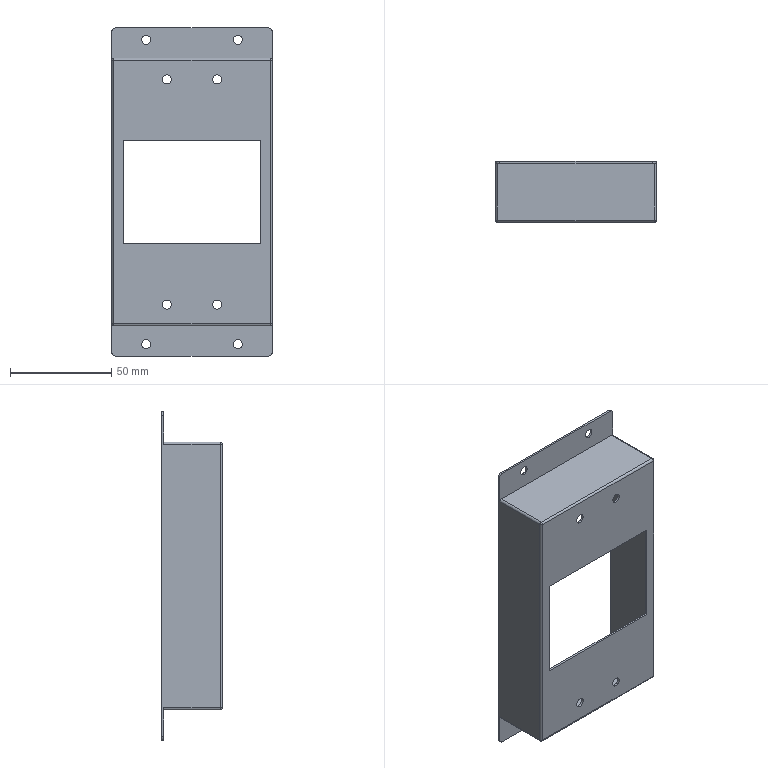Part | NX | 1 solid | 51 faces | box 79 x 30 x 162 mm | volume 21207 mm3 | cylinder 28 | plane 19 | sphere 4 | commonest cylinder face diameters 4.5 x16 2 x8 4 x4
STEP:
#1=CARTESIAN_POINT('',(38.5,0.,65.));
#2=VERTEX_POINT('',#1);
#3=CARTESIAN_POINT('',(-38.5,0.,65.));
#4=VERTEX_POINT('',#3);
#5=CARTESIAN_POINT('',(0.,0.,65.));
#6=DIRECTION('',(-1.,0.,0.));
#7=VECTOR('',#6,1000.);
#8=LINE('',#5,#7);
#9=EDGE_CURVE('',#2,#4,#8,.T.);
#10=ORIENTED_EDGE('',*,*,#9,.T.);
#11=CARTESIAN_POINT('',(-38.5,0.,-65.));
#12=VERTEX_POINT('',#11);
#13=CARTESIAN_POINT('',(-38.5,0.,0.));
#14=DIRECTION('',(0.,0.,-1.));
#15=VECTOR('',#14,1000.);
#16=LINE('',#13,#15);
#17=EDGE_CURVE('',#4,#12,#16,.T.);
#18=ORIENTED_EDGE('',*,*,#17,.T.);
#19=CARTESIAN_POINT('',(38.5,0.,-65.));
#20=VERTEX_POINT('',#19);
#21=CARTESIAN_POINT('',(0.,0.,-65.));
#22=DIRECTION('',(1.,0.,0.));
#23=VECTOR('',#22,1000.);
#24=LINE('',#21,#23);
#25=EDGE_CURVE('',#12,#20,#24,.T.);
#26=ORIENTED_EDGE('',*,*,#25,.T.);
#27=CARTESIAN_POINT('',(38.5,0.,0.));
#28=DIRECTION('',(0.,0.,1.));
#29=VECTOR('',#28,1000.);
#30=LINE('',#27,#29);
#31=EDGE_CURVE('',#20,#2,#30,.T.);
#32=ORIENTED_EDGE('',*,*,#31,.T.);
#33=EDGE_LOOP('',(#10,#18,#26,#32));
#34=FACE_BOUND('',#33,.T.);
#35=CARTESIAN_POINT('',(-14.75,0.,55.5));
#36=VERTEX_POINT('',#35);
#37=CARTESIAN_POINT('',(-10.25,0.,55.5));
#38=VERTEX_POINT('',#37);
#39=CARTESIAN_POINT('',(-12.5,0.,55.5));
#40=DIRECTION('',(0.,-1.,0.));
#41=DIRECTION('',(-1.,0.,0.));
#42=AXIS2_PLACEMENT_3D('',#39,#40,#41);
#43=CIRCLE('',#42,2.25);
#44=EDGE_CURVE('',#36,#38,#43,.T.);
#45=ORIENTED_EDGE('',*,*,#44,.F.);
#46=CARTESIAN_POINT('',(-12.5,0.,55.5));
#47=DIRECTION('',(0.,-1.,0.));
#48=DIRECTION('',(-1.,0.,0.));
#49=AXIS2_PLACEMENT_3D('',#46,#47,#48);
#50=CIRCLE('',#49,2.25);
#51=EDGE_CURVE('',#38,#36,#50,.T.);
#52=ORIENTED_EDGE('',*,*,#51,.F.);
#53=EDGE_LOOP('',(#45,#52));
#54=FACE_BOUND('',#53,.T.);
#55=CARTESIAN_POINT('',(10.25,0.,-55.5));
#56=VERTEX_POINT('',#55);
#57=CARTESIAN_POINT('',(14.75,0.,-55.5));
#58=VERTEX_POINT('',#57);
#59=CARTESIAN_POINT('',(12.5,0.,-55.5));
#60=DIRECTION('',(0.,-1.,0.));
#61=DIRECTION('',(-1.,0.,0.));
#62=AXIS2_PLACEMENT_3D('',#59,#60,#61);
#63=CIRCLE('',#62,2.25);
#64=EDGE_CURVE('',#56,#58,#63,.T.);
#65=ORIENTED_EDGE('',*,*,#64,.F.);
#66=CARTESIAN_POINT('',(12.5,0.,-55.5));
#67=DIRECTION('',(0.,-1.,0.));
#68=DIRECTION('',(-1.,0.,0.));
#69=AXIS2_PLACEMENT_3D('',#66,#67,#68);
#70=CIRCLE('',#69,2.25);
#71=EDGE_CURVE('',#58,#56,#70,.T.);
#72=ORIENTED_EDGE('',*,*,#71,.F.);
#73=EDGE_LOOP('',(#65,#72));
#74=FACE_BOUND('',#73,.T.);
#75=CARTESIAN_POINT('',(-34.,0.,25.5));
#76=VERTEX_POINT('',#75);
#77=CARTESIAN_POINT('',(-34.,0.,-25.5));
#78=VERTEX_POINT('',#77);
#79=CARTESIAN_POINT('',(-34.,0.,25.5));
#80=DIRECTION('',(0.,0.,-1.));
#81=VECTOR('',#80,1000.);
#82=LINE('',#79,#81);
#83=EDGE_CURVE('',#76,#78,#82,.T.);
#84=ORIENTED_EDGE('',*,*,#83,.F.);
#85=CARTESIAN_POINT('',(34.,0.,25.5));
#86=VERTEX_POINT('',#85);
#87=CARTESIAN_POINT('',(34.,0.,25.5));
#88=DIRECTION('',(-1.,0.,0.));
#89=VECTOR('',#88,1000.);
#90=LINE('',#87,#89);
#91=EDGE_CURVE('',#86,#76,#90,.T.);
#92=ORIENTED_EDGE('',*,*,#91,.F.);
#93=CARTESIAN_POINT('',(34.,0.,-25.5));
#94=VERTEX_POINT('',#93);
#95=CARTESIAN_POINT('',(34.,0.,-25.5));
#96=DIRECTION('',(0.,0.,1.));
#97=VECTOR('',#96,1000.);
#98=LINE('',#95,#97);
#99=EDGE_CURVE('',#94,#86,#98,.T.);
#100=ORIENTED_EDGE('',*,*,#99,.F.);
#101=CARTESIAN_POINT('',(-34.,0.,-25.5));
#102=DIRECTION('',(1.,0.,0.));
#103=VECTOR('',#102,1000.);
#104=LINE('',#101,#103);
#105=EDGE_CURVE('',#78,#94,#104,.T.);
#106=ORIENTED_EDGE('',*,*,#105,.F.);
#107=EDGE_LOOP('',(#84,#92,#100,#106));
#108=FACE_BOUND('',#107,.T.);
#109=CARTESIAN_POINT('',(-10.25,0.,-55.5));
#110=VERTEX_POINT('',#109);
#111=CARTESIAN_POINT('',(-14.75,0.,-55.5));
#112=VERTEX_POINT('',#111);
#113=CARTESIAN_POINT('',(-12.5,0.,-55.5));
#114=DIRECTION('',(0.,-1.,0.));
#115=DIRECTION('',(-1.,0.,0.));
#116=AXIS2_PLACEMENT_3D('',#113,#114,#115);
#117=CIRCLE('',#116,2.25);
#118=EDGE_CURVE('',#110,#112,#117,.T.);
#119=ORIENTED_EDGE('',*,*,#118,.F.);
#120=CARTESIAN_POINT('',(-12.5,0.,-55.5));
#121=DIRECTION('',(0.,-1.,0.));
#122=DIRECTION('',(-1.,0.,0.));
#123=AXIS2_PLACEMENT_3D('',#120,#121,#122);
#124=CIRCLE('',#123,2.25);
#125=EDGE_CURVE('',#112,#110,#124,.T.);
#126=ORIENTED_EDGE('',*,*,#125,.F.);
#127=EDGE_LOOP('',(#119,#126));
#128=FACE_BOUND('',#127,.T.);
#129=CARTESIAN_POINT('',(10.25,0.,55.5));
#130=VERTEX_POINT('',#129);
#131=CARTESIAN_POINT('',(14.75,0.,55.5));
#132=VERTEX_POINT('',#131);
#133=CARTESIAN_POINT('',(12.5,0.,55.5));
#134=DIRECTION('',(0.,-1.,0.));
#135=DIRECTION('',(-1.,0.,0.));
#136=AXIS2_PLACEMENT_3D('',#133,#134,#135);
#137=CIRCLE('',#136,2.25);
#138=EDGE_CURVE('',#130,#132,#137,.T.);
#139=ORIENTED_EDGE('',*,*,#138,.F.);
#140=CARTESIAN_POINT('',(12.5,0.,55.5));
#141=DIRECTION('',(0.,-1.,0.));
#142=DIRECTION('',(-1.,0.,0.));
#143=AXIS2_PLACEMENT_3D('',#140,#141,#142);
#144=CIRCLE('',#143,2.25);
#145=EDGE_CURVE('',#132,#130,#144,.T.);
#146=ORIENTED_EDGE('',*,*,#145,.F.);
#147=EDGE_LOOP('',(#139,#146));
#148=FACE_BOUND('',#147,.T.);
#149=CARTESIAN_POINT('',(0.,0.,0.));
#150=DIRECTION('',(0.,1.,0.));
#151=DIRECTION('',(1.,0.,0.));
#152=AXIS2_PLACEMENT_3D('',#149,#150,#151);
#153=PLANE('',#152);
#154=ADVANCED_FACE('',(#34,#54,#74,#108,#128,#148),#153,.F.);
#155=CARTESIAN_POINT('',(38.5,29.,66.));
#156=VERTEX_POINT('',#155);
#157=CARTESIAN_POINT('',(38.5,1.,66.));
#158=VERTEX_POINT('',#157);
#159=CARTESIAN_POINT('',(38.5,0.,66.));
#160=DIRECTION('',(0.,-1.,0.));
#161=VECTOR('',#160,1000.);
#162=LINE('',#159,#161);
#163=EDGE_CURVE('',#156,#158,#162,.T.);
#164=ORIENTED_EDGE('',*,*,#163,.F.);
#165=CARTESIAN_POINT('',(-38.5,29.,66.));
#166=VERTEX_POINT('',#165);
#167=CARTESIAN_POINT('',(39.5,29.,66.));
#168=DIRECTION('',(-1.,0.,0.));
#169=VECTOR('',#168,1000.);
#170=LINE('',#167,#169);
#171=EDGE_CURVE('',#156,#166,#170,.T.);
#172=ORIENTED_EDGE('',*,*,#171,.T.);
#173=CARTESIAN_POINT('',(-38.5,1.,66.));
#174=VERTEX_POINT('',#173);
#175=CARTESIAN_POINT('',(-38.5,0.,66.));
#176=DIRECTION('',(0.,-1.,0.));
#177=VECTOR('',#176,1000.);
#178=LINE('',#175,#177);
#179=EDGE_CURVE('',#166,#174,#178,.T.);
#180=ORIENTED_EDGE('',*,*,#179,.T.);
#181=CARTESIAN_POINT('',(0.,1.,66.));
#182=DIRECTION('',(-1.,0.,0.));
#183=VECTOR('',#182,1000.);
#184=LINE('',#181,#183);
#185=EDGE_CURVE('',#158,#174,#184,.T.);
#186=ORIENTED_EDGE('',*,*,#185,.F.);
#187=EDGE_LOOP('',(#164,#172,#180,#186));
#188=FACE_BOUND('',#187,.T.);
#189=CARTESIAN_POINT('',(-39.5,0.,66.));
#190=DIRECTION('',(0.,0.,1.));
#191=DIRECTION('',(1.,0.,0.));
#192=AXIS2_PLACEMENT_3D('',#189,#190,#191);
#193=PLANE('',#192);
#194=ADVANCED_FACE('',(#188),#193,.T.);
#195=ORIENTED_EDGE('',*,*,#171,.F.);
#196=CARTESIAN_POINT('',(39.5,29.,65.));
#197=VERTEX_POINT('',#196);
#198=CARTESIAN_POINT('',(38.5,29.,65.));
#199=DIRECTION('',(0.,-1.,0.));
#200=DIRECTION('',(-1.,0.,0.));
#201=AXIS2_PLACEMENT_3D('',#198,#199,#200);
#202=CIRCLE('',#201,1.);
#203=EDGE_CURVE('',#197,#156,#202,.T.);
#204=ORIENTED_EDGE('',*,*,#203,.F.);
#205=CARTESIAN_POINT('',(39.5,29.,79.));
#206=VERTEX_POINT('',#205);
#207=CARTESIAN_POINT('',(39.5,29.,81.));
#208=DIRECTION('',(0.,0.,-1.));
#209=VECTOR('',#208,1000.);
#210=LINE('',#207,#209);
#211=EDGE_CURVE('',#206,#197,#210,.T.);
#212=ORIENTED_EDGE('',*,*,#211,.F.);
#213=CARTESIAN_POINT('',(37.5,29.,81.));
#214=VERTEX_POINT('',#213);
#215=CARTESIAN_POINT('',(37.5,29.,79.));
#216=DIRECTION('',(0.,1.,0.));
#217=DIRECTION('',(1.,0.,0.));
#218=AXIS2_PLACEMENT_3D('',#215,#216,#217);
#219=CIRCLE('',#218,2.);
#220=EDGE_CURVE('',#214,#206,#219,.T.);
#221=ORIENTED_EDGE('',*,*,#220,.F.);
#222=CARTESIAN_POINT('',(-37.5,29.,81.));
#223=VERTEX_POINT('',#222);
#224=CARTESIAN_POINT('',(-39.5,29.,81.));
#225=DIRECTION('',(1.,0.,0.));
#226=VECTOR('',#225,1000.);
#227=LINE('',#224,#226);
#228=EDGE_CURVE('',#223,#214,#227,.T.);
#229=ORIENTED_EDGE('',*,*,#228,.F.);
#230=CARTESIAN_POINT('',(-39.5,29.,79.));
#231=VERTEX_POINT('',#230);
#232=CARTESIAN_POINT('',(-37.5,29.,79.));
#233=DIRECTION('',(0.,1.,0.));
#234=DIRECTION('',(1.,0.,0.));
#235=AXIS2_PLACEMENT_3D('',#232,#233,#234);
#236=CIRCLE('',#235,2.);
#237=EDGE_CURVE('',#231,#223,#236,.T.);
#238=ORIENTED_EDGE('',*,*,#237,.F.);
#239=CARTESIAN_POINT('',(-39.5,29.,65.));
#240=VERTEX_POINT('',#239);
#241=CARTESIAN_POINT('',(-39.5,29.,66.));
#242=DIRECTION('',(0.,0.,1.));
#243=VECTOR('',#242,1000.);
#244=LINE('',#241,#243);
#245=EDGE_CURVE('',#240,#231,#244,.T.);
#246=ORIENTED_EDGE('',*,*,#245,.F.);
#247=CARTESIAN_POINT('',(-38.5,29.,65.));
#248=DIRECTION('',(0.,-1.,0.));
#249=DIRECTION('',(-1.,0.,0.));
#250=AXIS2_PLACEMENT_3D('',#247,#248,#249);
#251=CIRCLE('',#250,1.);
#252=EDGE_CURVE('',#166,#240,#251,.T.);
#253=ORIENTED_EDGE('',*,*,#252,.F.);
#254=EDGE_LOOP('',(#195,#204,#212,#221,#229,#238,#246,#253));
#255=FACE_BOUND('',#254,.T.);
#256=CARTESIAN_POINT('',(20.25,29.,75.));
#257=VERTEX_POINT('',#256);
#258=CARTESIAN_POINT('',(24.75,29.,75.));
#259=VERTEX_POINT('',#258);
#260=CARTESIAN_POINT('',(22.5,29.,75.));
#261=DIRECTION('',(0.,-1.,0.));
#262=DIRECTION('',(-1.,0.,0.));
#263=AXIS2_PLACEMENT_3D('',#260,#261,#262);
#264=CIRCLE('',#263,2.25);
#265=EDGE_CURVE('',#257,#259,#264,.T.);
#266=ORIENTED_EDGE('',*,*,#265,.F.);
#267=CARTESIAN_POINT('',(22.5,29.,75.));
#268=DIRECTION('',(0.,-1.,0.));
#269=DIRECTION('',(-1.,0.,0.));
#270=AXIS2_PLACEMENT_3D('',#267,#268,#269);
#271=CIRCLE('',#270,2.25);
#272=EDGE_CURVE('',#259,#257,#271,.T.);
#273=ORIENTED_EDGE('',*,*,#272,.F.);
#274=EDGE_LOOP('',(#266,#273));
#275=FACE_BOUND('',#274,.T.);
#276=CARTESIAN_POINT('',(-20.25,29.,75.));
#277=VERTEX_POINT('',#276);
#278=CARTESIAN_POINT('',(-24.75,29.,75.));
#279=VERTEX_POINT('',#278);
#280=CARTESIAN_POINT('',(-22.5,29.,75.));
#281=DIRECTION('',(0.,-1.,0.));
#282=DIRECTION('',(-1.,0.,0.));
#283=AXIS2_PLACEMENT_3D('',#280,#281,#282);
#284=CIRCLE('',#283,2.25);
#285=EDGE_CURVE('',#277,#279,#284,.T.);
#286=ORIENTED_EDGE('',*,*,#285,.F.);
#287=CARTESIAN_POINT('',(-22.5,29.,75.));
#288=DIRECTION('',(0.,-1.,0.));
#289=DIRECTION('',(-1.,0.,0.));
#290=AXIS2_PLACEMENT_3D('',#287,#288,#289);
#291=CIRCLE('',#290,2.25);
#292=EDGE_CURVE('',#279,#277,#291,.T.);
#293=ORIENTED_EDGE('',*,*,#292,.F.);
#294=EDGE_LOOP('',(#286,#293));
#295=FACE_BOUND('',#294,.T.);
#296=CARTESIAN_POINT('',(0.,29.,0.));
#297=DIRECTION('',(0.,-1.,0.));
#298=DIRECTION('',(0.,0.,-1.));
#299=AXIS2_PLACEMENT_3D('',#296,#297,#298);
#300=PLANE('',#299);
#301=ADVANCED_FACE('',(#255,#275,#295),#300,.T.);
#302=CARTESIAN_POINT('',(-39.5,29.,-65.));
#303=VERTEX_POINT('',#302);
#304=CARTESIAN_POINT('',(-39.5,1.,-65.));
#305=VERTEX_POINT('',#304);
#306=CARTESIAN_POINT('',(-39.5,0.,-65.));
#307=DIRECTION('',(0.,-1.,0.));
#308=VECTOR('',#307,1000.);
#309=LINE('',#306,#308);
#310=EDGE_CURVE('',#303,#305,#309,.T.);
#311=ORIENTED_EDGE('',*,*,#310,.T.);
#312=CARTESIAN_POINT('',(-39.5,1.,65.));
#313=VERTEX_POINT('',#312);
#314=CARTESIAN_POINT('',(-39.5,1.,0.));
#315=DIRECTION('',(0.,0.,-1.));
#316=VECTOR('',#315,1000.);
#317=LINE('',#314,#316);
#318=EDGE_CURVE('',#313,#305,#317,.T.);
#319=ORIENTED_EDGE('',*,*,#318,.F.);
#320=CARTESIAN_POINT('',(-39.5,0.,65.));
#321=DIRECTION('',(0.,-1.,0.));
#322=VECTOR('',#321,1000.);
#323=LINE('',#320,#322);
#324=EDGE_CURVE('',#240,#313,#323,.T.);
#325=ORIENTED_EDGE('',*,*,#324,.F.);
#326=ORIENTED_EDGE('',*,*,#245,.T.);
#327=CARTESIAN_POINT('',(-39.5,30.,79.));
#328=VERTEX_POINT('',#327);
#329=CARTESIAN_POINT('',(-39.5,0.,79.));
#330=DIRECTION('',(0.,1.,0.));
#331=VECTOR('',#330,1000.);
#332=LINE('',#329,#331);
#333=EDGE_CURVE('',#231,#328,#332,.T.);
#334=ORIENTED_EDGE('',*,*,#333,.T.);
#335=CARTESIAN_POINT('',(-39.5,30.,-79.));
#336=VERTEX_POINT('',#335);
#337=CARTESIAN_POINT('',(-39.5,30.,81.));
#338=DIRECTION('',(0.,0.,-1.));
#339=VECTOR('',#338,1000.);
#340=LINE('',#337,#339);
#341=EDGE_CURVE('',#328,#336,#340,.T.);
#342=ORIENTED_EDGE('',*,*,#341,.T.);
#343=CARTESIAN_POINT('',(-39.5,29.,-79.));
#344=VERTEX_POINT('',#343);
#345=CARTESIAN_POINT('',(-39.5,0.,-79.));
#346=DIRECTION('',(0.,1.,0.));
#347=VECTOR('',#346,1000.);
#348=LINE('',#345,#347);
#349=EDGE_CURVE('',#344,#336,#348,.T.);
#350=ORIENTED_EDGE('',*,*,#349,.F.);
#351=CARTESIAN_POINT('',(-39.5,29.,-81.));
#352=DIRECTION('',(0.,0.,1.));
#353=VECTOR('',#352,1000.);
#354=LINE('',#351,#353);
#355=EDGE_CURVE('',#344,#303,#354,.T.);
#356=ORIENTED_EDGE('',*,*,#355,.T.);
#357=EDGE_LOOP('',(#311,#319,#325,#326,#334,#342,#350,#356));
#358=FACE_BOUND('',#357,.T.);
#359=CARTESIAN_POINT('',(-39.5,0.,-66.));
#360=DIRECTION('',(-1.,0.,0.));
#361=DIRECTION('',(0.,0.,1.));
#362=AXIS2_PLACEMENT_3D('',#359,#360,#361);
#363=PLANE('',#362);
#364=ADVANCED_FACE('',(#358),#363,.T.);
#365=CARTESIAN_POINT('',(39.5,30.,-79.));
#366=VERTEX_POINT('',#365);
#367=CARTESIAN_POINT('',(39.5,30.,79.));
#368=VERTEX_POINT('',#367);
#369=CARTESIAN_POINT('',(39.5,30.,-81.));
#370=DIRECTION('',(0.,0.,1.));
#371=VECTOR('',#370,1000.);
#372=LINE('',#369,#371);
#373=EDGE_CURVE('',#366,#368,#372,.T.);
#374=ORIENTED_EDGE('',*,*,#373,.F.);
#375=CARTESIAN_POINT('',(37.5,30.,-81.));
#376=VERTEX_POINT('',#375);
#377=CARTESIAN_POINT('',(37.5,30.,-79.));
#378=DIRECTION('',(0.,1.,0.));
#379=DIRECTION('',(1.,0.,0.));
#380=AXIS2_PLACEMENT_3D('',#377,#378,#379);
#381=CIRCLE('',#380,2.);
#382=EDGE_CURVE('',#366,#376,#381,.T.);
#383=ORIENTED_EDGE('',*,*,#382,.T.);
#384=CARTESIAN_POINT('',(-37.5,30.,-81.));
#385=VERTEX_POINT('',#384);
#386=CARTESIAN_POINT('',(39.5,30.,-81.));
#387=DIRECTION('',(-1.,0.,0.));
#388=VECTOR('',#387,1000.);
#389=LINE('',#386,#388);
#390=EDGE_CURVE('',#376,#385,#389,.T.);
#391=ORIENTED_EDGE('',*,*,#390,.T.);
#392=CARTESIAN_POINT('',(-37.5,30.,-79.));
#393=DIRECTION('',(0.,1.,0.));
#394=DIRECTION('',(1.,0.,0.));
#395=AXIS2_PLACEMENT_3D('',#392,#393,#394);
#396=CIRCLE('',#395,2.);
#397=EDGE_CURVE('',#385,#336,#396,.T.);
#398=ORIENTED_EDGE('',*,*,#397,.T.);
#399=ORIENTED_EDGE('',*,*,#341,.F.);
#400=CARTESIAN_POINT('',(-37.5,30.,81.));
#401=VERTEX_POINT('',#400);
#402=CARTESIAN_POINT('',(-37.5,30.,79.));
#403=DIRECTION('',(0.,1.,0.));
#404=DIRECTION('',(1.,0.,0.));
#405=AXIS2_PLACEMENT_3D('',#402,#403,#404);
#406=CIRCLE('',#405,2.);
#407=EDGE_CURVE('',#328,#401,#406,.T.);
#408=ORIENTED_EDGE('',*,*,#407,.T.);
#409=CARTESIAN_POINT('',(37.5,30.,81.));
#410=VERTEX_POINT('',#409);
#411=CARTESIAN_POINT('',(-39.5,30.,81.));
#412=DIRECTION('',(1.,0.,0.));
#413=VECTOR('',#412,1000.);
#414=LINE('',#411,#413);
#415=EDGE_CURVE('',#401,#410,#414,.T.);
#416=ORIENTED_EDGE('',*,*,#415,.T.);
#417=CARTESIAN_POINT('',(37.5,30.,79.));
#418=DIRECTION('',(0.,1.,0.));
#419=DIRECTION('',(1.,0.,0.));
#420=AXIS2_PLACEMENT_3D('',#417,#418,#419);
#421=CIRCLE('',#420,2.);
#422=EDGE_CURVE('',#410,#368,#421,.T.);
#423=ORIENTED_EDGE('',*,*,#422,.T.);
#424=EDGE_LOOP('',(#374,#383,#391,#398,#399,#408,#416,#423));
#425=FACE_BOUND('',#424,.T.);
#426=CARTESIAN_POINT('',(38.5,30.,65.));
#427=VERTEX_POINT('',#426);
#428=CARTESIAN_POINT('',(-38.5,30.,65.));
#429=VERTEX_POINT('',#428);
#430=CARTESIAN_POINT('',(38.5,30.,65.));
#431=DIRECTION('',(-1.,0.,0.));
#432=VECTOR('',#431,1000.);
#433=LINE('',#430,#432);
#434=EDGE_CURVE('',#427,#429,#433,.T.);
#435=ORIENTED_EDGE('',*,*,#434,.T.);
#436=CARTESIAN_POINT('',(-38.5,30.,-65.));
#437=VERTEX_POINT('',#436);
#438=CARTESIAN_POINT('',(-38.5,30.,65.));
#439=DIRECTION('',(0.,0.,-1.));
#440=VECTOR('',#439,1000.);
#441=LINE('',#438,#440);
#442=EDGE_CURVE('',#429,#437,#441,.T.);
#443=ORIENTED_EDGE('',*,*,#442,.T.);
#444=CARTESIAN_POINT('',(38.5,30.,-65.));
#445=VERTEX_POINT('',#444);
#446=CARTESIAN_POINT('',(-38.5,30.,-65.));
#447=DIRECTION('',(1.,0.,0.));
#448=VECTOR('',#447,1000.);
#449=LINE('',#446,#448);
#450=EDGE_CURVE('',#437,#445,#449,.T.);
#451=ORIENTED_EDGE('',*,*,#450,.T.);
#452=CARTESIAN_POINT('',(38.5,30.,-65.));
#453=DIRECTION('',(0.,0.,1.));
#454=VECTOR('',#453,1000.);
#455=LINE('',#452,#454);
#456=EDGE_CURVE('',#445,#427,#455,.T.);
#457=ORIENTED_EDGE('',*,*,#456,.T.);
#458=EDGE_LOOP('',(#435,#443,#451,#457));
#459=FACE_BOUND('',#458,.T.);
#460=CARTESIAN_POINT('',(-20.25,30.,-75.));
#461=VERTEX_POINT('',#460);
#462=CARTESIAN_POINT('',(-24.75,30.,-75.));
#463=VERTEX_POINT('',#462);
#464=CARTESIAN_POINT('',(-22.5,30.,-75.));
#465=DIRECTION('',(0.,1.,0.));
#466=DIRECTION('',(1.,0.,0.));
#467=AXIS2_PLACEMENT_3D('',#464,#465,#466);
#468=CIRCLE('',#467,2.25);
#469=EDGE_CURVE('',#461,#463,#468,.T.);
#470=ORIENTED_EDGE('',*,*,#469,.F.);
#471=CARTESIAN_POINT('',(-22.5,30.,-75.));
#472=DIRECTION('',(0.,1.,0.));
#473=DIRECTION('',(1.,0.,0.));
#474=AXIS2_PLACEMENT_3D('',#471,#472,#473);
#475=CIRCLE('',#474,2.25);
#476=EDGE_CURVE('',#463,#461,#475,.T.);
#477=ORIENTED_EDGE('',*,*,#476,.F.);
#478=EDGE_LOOP('',(#470,#477));
#479=FACE_BOUND('',#478,.T.);
#480=CARTESIAN_POINT('',(24.75,30.,75.));
#481=VERTEX_POINT('',#480);
#482=CARTESIAN_POINT('',(20.25,30.,75.));
#483=VERTEX_POINT('',#482);
#484=CARTESIAN_POINT('',(22.5,30.,75.));
#485=DIRECTION('',(0.,1.,0.));
#486=DIRECTION('',(1.,0.,0.));
#487=AXIS2_PLACEMENT_3D('',#484,#485,#486);
#488=CIRCLE('',#487,2.25);
#489=EDGE_CURVE('',#481,#483,#488,.T.);
#490=ORIENTED_EDGE('',*,*,#489,.F.);
#491=CARTESIAN_POINT('',(22.5,30.,75.));
#492=DIRECTION('',(0.,1.,0.));
#493=DIRECTION('',(1.,0.,0.));
#494=AXIS2_PLACEMENT_3D('',#491,#492,#493);
#495=CIRCLE('',#494,2.25);
#496=EDGE_CURVE('',#483,#481,#495,.T.);
#497=ORIENTED_EDGE('',*,*,#496,.F.);
#498=EDGE_LOOP('',(#490,#497));
#499=FACE_BOUND('',#498,.T.);
#500=CARTESIAN_POINT('',(-20.25,30.,75.));
#501=VERTEX_POINT('',#500);
#502=CARTESIAN_POINT('',(-24.75,30.,75.));
#503=VERTEX_POINT('',#502);
#504=CARTESIAN_POINT('',(-22.5,30.,75.));
#505=DIRECTION('',(0.,1.,0.));
#506=DIRECTION('',(1.,0.,0.));
#507=AXIS2_PLACEMENT_3D('',#504,#505,#506);
#508=CIRCLE('',#507,2.25);
#509=EDGE_CURVE('',#501,#503,#508,.T.);
#510=ORIENTED_EDGE('',*,*,#509,.F.);
#511=CARTESIAN_POINT('',(-22.5,30.,75.));
#512=DIRECTION('',(0.,1.,0.));
#513=DIRECTION('',(1.,0.,0.));
#514=AXIS2_PLACEMENT_3D('',#511,#512,#513);
#515=CIRCLE('',#514,2.25);
#516=EDGE_CURVE('',#503,#501,#515,.T.);
#517=ORIENTED_EDGE('',*,*,#516,.F.);
#518=EDGE_LOOP('',(#510,#517));
#519=FACE_BOUND('',#518,.T.);
#520=CARTESIAN_POINT('',(24.75,30.,-75.));
#521=VERTEX_POINT('',#520);
#522=CARTESIAN_POINT('',(20.25,30.,-75.));
#523=VERTEX_POINT('',#522);
#524=CARTESIAN_POINT('',(22.5,30.,-75.));
#525=DIRECTION('',(0.,1.,0.));
#526=DIRECTION('',(1.,0.,0.));
#527=AXIS2_PLACEMENT_3D('',#524,#525,#526);
#528=CIRCLE('',#527,2.25);
#529=EDGE_CURVE('',#521,#523,#528,.T.);
#530=ORIENTED_EDGE('',*,*,#529,.F.);
#531=CARTESIAN_POINT('',(22.5,30.,-75.));
#532=DIRECTION('',(0.,1.,0.));
#533=DIRECTION('',(1.,0.,0.));
#534=AXIS2_PLACEMENT_3D('',#531,#532,#533);
#535=CIRCLE('',#534,2.25);
#536=EDGE_CURVE('',#523,#521,#535,.T.);
#537=ORIENTED_EDGE('',*,*,#536,.F.);
#538=EDGE_LOOP('',(#530,#537));
#539=FACE_BOUND('',#538,.T.);
#540=CARTESIAN_POINT('',(0.,30.,0.));
#541=DIRECTION('',(0.,1.,0.));
#542=DIRECTION('',(1.,0.,0.));
#543=AXIS2_PLACEMENT_3D('',#540,#541,#542);
#544=PLANE('',#543);
#545=ADVANCED_FACE('',(#425,#459,#479,#499,#519,#539),#544,.T.);
#546=CARTESIAN_POINT('',(39.5,29.,-65.));
#547=VERTEX_POINT('',#546);
#548=CARTESIAN_POINT('',(39.5,1.,-65.));
#549=VERTEX_POINT('',#548);
#550=CARTESIAN_POINT('',(39.5,0.,-65.));
#551=DIRECTION('',(0.,-1.,0.));
#552=VECTOR('',#551,1000.);
#553=LINE('',#550,#552);
#554=EDGE_CURVE('',#547,#549,#553,.T.);
#555=ORIENTED_EDGE('',*,*,#554,.F.);
#556=CARTESIAN_POINT('',(39.5,29.,-79.));
#557=VERTEX_POINT('',#556);
#558=CARTESIAN_POINT('',(39.5,29.,-66.));
#559=DIRECTION('',(0.,0.,-1.));
#560=VECTOR('',#559,1000.);
#561=LINE('',#558,#560);
#562=EDGE_CURVE('',#547,#557,#561,.T.);
#563=ORIENTED_EDGE('',*,*,#562,.T.);
#564=CARTESIAN_POINT('',(39.5,0.,-79.));
#565=DIRECTION('',(0.,1.,0.));
#566=VECTOR('',#565,1000.);
#567=LINE('',#564,#566);
#568=EDGE_CURVE('',#557,#366,#567,.T.);
#569=ORIENTED_EDGE('',*,*,#568,.T.);
#570=ORIENTED_EDGE('',*,*,#373,.T.);
#571=CARTESIAN_POINT('',(39.5,0.,79.));
#572=DIRECTION('',(0.,1.,0.));
#573=VECTOR('',#572,1000.);
#574=LINE('',#571,#573);
#575=EDGE_CURVE('',#206,#368,#574,.T.);
#576=ORIENTED_EDGE('',*,*,#575,.F.);
#577=ORIENTED_EDGE('',*,*,#211,.T.);
#578=CARTESIAN_POINT('',(39.5,1.,65.));
#579=VERTEX_POINT('',#578);
#580=CARTESIAN_POINT('',(39.5,0.,65.));
#581=DIRECTION('',(0.,-1.,0.));
#582=VECTOR('',#581,1000.);
#583=LINE('',#580,#582);
#584=EDGE_CURVE('',#197,#579,#583,.T.);
#585=ORIENTED_EDGE('',*,*,#584,.T.);
#586=CARTESIAN_POINT('',(39.5,1.,0.));
#587=DIRECTION('',(0.,0.,1.));
#588=VECTOR('',#587,1000.);
#589=LINE('',#586,#588);
#590=EDGE_CURVE('',#549,#579,#589,.T.);
#591=ORIENTED_EDGE('',*,*,#590,.F.);
#592=EDGE_LOOP('',(#555,#563,#569,#570,#576,#577,#585,#591));
#593=FACE_BOUND('',#592,.T.);
#594=CARTESIAN_POINT('',(39.5,0.,66.));
#595=DIRECTION('',(1.,0.,0.));
#596=DIRECTION('',(0.,1.,0.));
#597=AXIS2_PLACEMENT_3D('',#594,#595,#596);
#598=PLANE('',#597);
#599=ADVANCED_FACE('',(#593),#598,.T.);
#600=ORIENTED_EDGE('',*,*,#415,.F.);
#601=CARTESIAN_POINT('',(-37.5,0.,81.));
#602=DIRECTION('',(0.,1.,0.));
#603=VECTOR('',#602,1000.);
#604=LINE('',#601,#603);
#605=EDGE_CURVE('',#223,#401,#604,.T.);
#606=ORIENTED_EDGE('',*,*,#605,.F.);
#607=ORIENTED_EDGE('',*,*,#228,.T.);
#608=CARTESIAN_POINT('',(37.5,0.,81.));
#609=DIRECTION('',(0.,1.,0.));
#610=VECTOR('',#609,1000.);
#611=LINE('',#608,#610);
#612=EDGE_CURVE('',#214,#410,#611,.T.);
#613=ORIENTED_EDGE('',*,*,#612,.T.);
#614=EDGE_LOOP('',(#600,#606,#607,#613));
#615=FACE_BOUND('',#614,.T.);
#616=CARTESIAN_POINT('',(39.5,30.,81.));
#617=DIRECTION('',(0.,0.,1.));
#618=DIRECTION('',(1.,0.,0.));
#619=AXIS2_PLACEMENT_3D('',#616,#617,#618);
#620=PLANE('',#619);
#621=ADVANCED_FACE('',(#615),#620,.T.);
#622=ORIENTED_EDGE('',*,*,#390,.F.);
#623=CARTESIAN_POINT('',(37.5,29.,-81.));
#624=VERTEX_POINT('',#623);
#625=CARTESIAN_POINT('',(37.5,0.,-81.));
#626=DIRECTION('',(0.,1.,0.));
#627=VECTOR('',#626,1000.);
#628=LINE('',#625,#627);
#629=EDGE_CURVE('',#624,#376,#628,.T.);
#630=ORIENTED_EDGE('',*,*,#629,.F.);
#631=CARTESIAN_POINT('',(-37.5,29.,-81.));
#632=VERTEX_POINT('',#631);
#633=CARTESIAN_POINT('',(39.5,29.,-81.));
#634=DIRECTION('',(-1.,0.,0.));
#635=VECTOR('',#634,1000.);
#636=LINE('',#633,#635);
#637=EDGE_CURVE('',#624,#632,#636,.T.);
#638=ORIENTED_EDGE('',*,*,#637,.T.);
#639=CARTESIAN_POINT('',(-37.5,0.,-81.));
#640=DIRECTION('',(0.,1.,0.));
#641=VECTOR('',#640,1000.);
#642=LINE('',#639,#641);
#643=EDGE_CURVE('',#632,#385,#642,.T.);
#644=ORIENTED_EDGE('',*,*,#643,.T.);
#645=EDGE_LOOP('',(#622,#630,#638,#644));
#646=FACE_BOUND('',#645,.T.);
#647=CARTESIAN_POINT('',(-39.5,30.,-81.));
#648=DIRECTION('',(0.,0.,-1.));
#649=DIRECTION('',(0.,-1.,0.));
#650=AXIS2_PLACEMENT_3D('',#647,#648,#649);
#651=PLANE('',#650);
#652=ADVANCED_FACE('',(#646),#651,.T.);
#653=CARTESIAN_POINT('',(-38.5,29.,-66.));
#654=VERTEX_POINT('',#653);
#655=CARTESIAN_POINT('',(38.5,29.,-66.));
#656=VERTEX_POINT('',#655);
#657=CARTESIAN_POINT('',(-39.5,29.,-66.));
#658=DIRECTION('',(1.,0.,0.));
#659=VECTOR('',#658,1000.);
#660=LINE('',#657,#659);
#661=EDGE_CURVE('',#654,#656,#660,.T.);
#662=ORIENTED_EDGE('',*,*,#661,.F.);
#663=CARTESIAN_POINT('',(-38.5,29.,-65.));
#664=DIRECTION('',(0.,-1.,0.));
#665=DIRECTION('',(-1.,0.,0.));
#666=AXIS2_PLACEMENT_3D('',#663,#664,#665);
#667=CIRCLE('',#666,1.);
#668=EDGE_CURVE('',#303,#654,#667,.T.);
#669=ORIENTED_EDGE('',*,*,#668,.F.);
#670=ORIENTED_EDGE('',*,*,#355,.F.);
#671=CARTESIAN_POINT('',(-37.5,29.,-79.));
#672=DIRECTION('',(0.,1.,0.));
#673=DIRECTION('',(1.,0.,0.));
#674=AXIS2_PLACEMENT_3D('',#671,#672,#673);
#675=CIRCLE('',#674,2.);
#676=EDGE_CURVE('',#632,#344,#675,.T.);
#677=ORIENTED_EDGE('',*,*,#676,.F.);
#678=ORIENTED_EDGE('',*,*,#637,.F.);
#679=CARTESIAN_POINT('',(37.5,29.,-79.));
#680=DIRECTION('',(0.,1.,0.));
#681=DIRECTION('',(1.,0.,0.));
#682=AXIS2_PLACEMENT_3D('',#679,#680,#681);
#683=CIRCLE('',#682,2.);
#684=EDGE_CURVE('',#557,#624,#683,.T.);
#685=ORIENTED_EDGE('',*,*,#684,.F.);
#686=ORIENTED_EDGE('',*,*,#562,.F.);
#687=CARTESIAN_POINT('',(38.5,29.,-65.));
#688=DIRECTION('',(0.,-1.,0.));
#689=DIRECTION('',(-1.,0.,0.));
#690=AXIS2_PLACEMENT_3D('',#687,#688,#689);
#691=CIRCLE('',#690,1.);
#692=EDGE_CURVE('',#656,#547,#691,.T.);
#693=ORIENTED_EDGE('',*,*,#692,.F.);
#694=EDGE_LOOP('',(#662,#669,#670,#677,#678,#685,#686,#693));
#695=FACE_BOUND('',#694,.T.);
#696=CARTESIAN_POINT('',(-20.25,29.,-75.));
#697=VERTEX_POINT('',#696);
#698=CARTESIAN_POINT('',(-24.75,29.,-75.));
#699=VERTEX_POINT('',#698);
#700=CARTESIAN_POINT('',(-22.5,29.,-75.));
#701=DIRECTION('',(0.,-1.,0.));
#702=DIRECTION('',(-1.,0.,0.));
#703=AXIS2_PLACEMENT_3D('',#700,#701,#702);
#704=CIRCLE('',#703,2.25);
#705=EDGE_CURVE('',#697,#699,#704,.T.);
#706=ORIENTED_EDGE('',*,*,#705,.F.);
#707=CARTESIAN_POINT('',(-22.5,29.,-75.));
#708=DIRECTION('',(0.,-1.,0.));
#709=DIRECTION('',(-1.,0.,0.));
#710=AXIS2_PLACEMENT_3D('',#707,#708,#709);
#711=CIRCLE('',#710,2.25);
#712=EDGE_CURVE('',#699,#697,#711,.T.);
#713=ORIENTED_EDGE('',*,*,#712,.F.);
#714=EDGE_LOOP('',(#706,#713));
#715=FACE_BOUND('',#714,.T.);
#716=CARTESIAN_POINT('',(24.75,29.,-75.));
#717=VERTEX_POINT('',#716);
#718=CARTESIAN_POINT('',(20.25,29.,-75.));
#719=VERTEX_POINT('',#718);
#720=CARTESIAN_POINT('',(22.5,29.,-75.));
#721=DIRECTION('',(0.,-1.,0.));
#722=DIRECTION('',(-1.,0.,0.));
#723=AXIS2_PLACEMENT_3D('',#720,#721,#722);
#724=CIRCLE('',#723,2.25);
#725=EDGE_CURVE('',#717,#719,#724,.T.);
#726=ORIENTED_EDGE('',*,*,#725,.F.);
#727=CARTESIAN_POINT('',(22.5,29.,-75.));
#728=DIRECTION('',(0.,-1.,0.));
#729=DIRECTION('',(-1.,0.,0.));
#730=AXIS2_PLACEMENT_3D('',#727,#728,#729);
#731=CIRCLE('',#730,2.25);
#732=EDGE_CURVE('',#719,#717,#731,.T.);
#733=ORIENTED_EDGE('',*,*,#732,.F.);
#734=EDGE_LOOP('',(#726,#733));
#735=FACE_BOUND('',#734,.T.);
#736=CARTESIAN_POINT('',(0.,29.,0.));
#737=DIRECTION('',(0.,-1.,0.));
#738=DIRECTION('',(0.,0.,-1.));
#739=AXIS2_PLACEMENT_3D('',#736,#737,#738);
#740=PLANE('',#739);
#741=ADVANCED_FACE('',(#695,#715,#735),#740,.T.);
#742=ORIENTED_EDGE('',*,*,#661,.T.);
#743=CARTESIAN_POINT('',(38.5,1.,-66.));
#744=VERTEX_POINT('',#743);
#745=CARTESIAN_POINT('',(38.5,0.,-66.));
#746=DIRECTION('',(0.,-1.,0.));
#747=VECTOR('',#746,1000.);
#748=LINE('',#745,#747);
#749=EDGE_CURVE('',#656,#744,#748,.T.);
#750=ORIENTED_EDGE('',*,*,#749,.T.);
#751=CARTESIAN_POINT('',(-38.5,1.,-66.));
#752=VERTEX_POINT('',#751);
#753=CARTESIAN_POINT('',(0.,1.,-66.));
#754=DIRECTION('',(1.,0.,0.));
#755=VECTOR('',#754,1000.);
#756=LINE('',#753,#755);
#757=EDGE_CURVE('',#752,#744,#756,.T.);
#758=ORIENTED_EDGE('',*,*,#757,.F.);
#759=CARTESIAN_POINT('',(-38.5,0.,-66.));
#760=DIRECTION('',(0.,-1.,0.));
#761=VECTOR('',#760,1000.);
#762=LINE('',#759,#761);
#763=EDGE_CURVE('',#654,#752,#762,.T.);
#764=ORIENTED_EDGE('',*,*,#763,.F.);
#765=EDGE_LOOP('',(#742,#750,#758,#764));
#766=FACE_BOUND('',#765,.T.);
#767=CARTESIAN_POINT('',(39.5,0.,-66.));
#768=DIRECTION('',(0.,0.,-1.));
#769=DIRECTION('',(0.,-1.,0.));
#770=AXIS2_PLACEMENT_3D('',#767,#768,#769);
#771=PLANE('',#770);
#772=ADVANCED_FACE('',(#766),#771,.T.);
#773=ORIENTED_EDGE('',*,*,#725,.T.);
#774=CARTESIAN_POINT('',(20.25,30.,-75.));
#775=DIRECTION('',(0.,-1.,0.));
#776=VECTOR('',#775,1000.);
#777=LINE('',#774,#776);
#778=EDGE_CURVE('',#719,#523,#777,.F.);
#779=ORIENTED_EDGE('',*,*,#778,.T.);
#780=ORIENTED_EDGE('',*,*,#536,.T.);
#781=CARTESIAN_POINT('',(24.75,30.,-75.));
#782=DIRECTION('',(0.,-1.,0.));
#783=VECTOR('',#782,1000.);
#784=LINE('',#781,#783);
#785=EDGE_CURVE('',#717,#521,#784,.F.);
#786=ORIENTED_EDGE('',*,*,#785,.F.);
#787=EDGE_LOOP('',(#773,#779,#780,#786));
#788=FACE_BOUND('',#787,.T.);
#789=CARTESIAN_POINT('',(22.5,30.,-75.));
#790=DIRECTION('',(0.,-1.,0.));
#791=DIRECTION('',(1.,0.,0.));
#792=AXIS2_PLACEMENT_3D('',#789,#790,#791);
#793=CYLINDRICAL_SURFACE('',#792,2.25);
#794=ADVANCED_FACE('',(#788),#793,.F.);
#795=ORIENTED_EDGE('',*,*,#83,.T.);
#796=CARTESIAN_POINT('',(-34.,1.,-25.5));
#797=VERTEX_POINT('',#796);
#798=CARTESIAN_POINT('',(-34.,0.,-25.5));
#799=DIRECTION('',(0.,1.,0.));
#800=VECTOR('',#799,1000.);
#801=LINE('',#798,#800);
#802=EDGE_CURVE('',#78,#797,#801,.T.);
#803=ORIENTED_EDGE('',*,*,#802,.T.);
#804=CARTESIAN_POINT('',(-34.,1.,25.5));
#805=VERTEX_POINT('',#804);
#806=CARTESIAN_POINT('',(-34.,1.,25.5));
#807=DIRECTION('',(0.,0.,-1.));
#808=VECTOR('',#807,1000.);
#809=LINE('',#806,#808);
#810=EDGE_CURVE('',#805,#797,#809,.T.);
#811=ORIENTED_EDGE('',*,*,#810,.F.);
#812=CARTESIAN_POINT('',(-34.,0.,25.5));
#813=DIRECTION('',(0.,1.,0.));
#814=VECTOR('',#813,1000.);
#815=LINE('',#812,#814);
#816=EDGE_CURVE('',#76,#805,#815,.T.);
#817=ORIENTED_EDGE('',*,*,#816,.F.);
#818=EDGE_LOOP('',(#795,#803,#811,#817));
#819=FACE_BOUND('',#818,.T.);
#820=CARTESIAN_POINT('',(-34.,1.,-25.5));
#821=DIRECTION('',(-1.,0.,0.));
#822=DIRECTION('',(0.,0.,1.));
#823=AXIS2_PLACEMENT_3D('',#820,#821,#822);
#824=PLANE('',#823);
#825=ADVANCED_FACE('',(#819),#824,.F.);
#826=ORIENTED_EDGE('',*,*,#705,.T.);
#827=CARTESIAN_POINT('',(-24.75,30.,-75.));
#828=DIRECTION('',(0.,-1.,0.));
#829=VECTOR('',#828,1000.);
#830=LINE('',#827,#829);
#831=EDGE_CURVE('',#699,#463,#830,.F.);
#832=ORIENTED_EDGE('',*,*,#831,.T.);
#833=ORIENTED_EDGE('',*,*,#476,.T.);
#834=CARTESIAN_POINT('',(-20.25,30.,-75.));
#835=DIRECTION('',(0.,-1.,0.));
#836=VECTOR('',#835,1000.);
#837=LINE('',#834,#836);
#838=EDGE_CURVE('',#697,#461,#837,.F.);
#839=ORIENTED_EDGE('',*,*,#838,.F.);
#840=EDGE_LOOP('',(#826,#832,#833,#839));
#841=FACE_BOUND('',#840,.T.);
#842=CARTESIAN_POINT('',(-22.5,30.,-75.));
#843=DIRECTION('',(0.,-1.,0.));
#844=DIRECTION('',(1.,0.,0.));
#845=AXIS2_PLACEMENT_3D('',#842,#843,#844);
#846=CYLINDRICAL_SURFACE('',#845,2.25);
#847=ADVANCED_FACE('',(#841),#846,.F.);
#848=ORIENTED_EDGE('',*,*,#99,.T.);
#849=CARTESIAN_POINT('',(34.,1.,25.5));
#850=VERTEX_POINT('',#849);
#851=CARTESIAN_POINT('',(34.,0.,25.5));
#852=DIRECTION('',(0.,1.,0.));
#853=VECTOR('',#852,1000.);
#854=LINE('',#851,#853);
#855=EDGE_CURVE('',#86,#850,#854,.T.);
#856=ORIENTED_EDGE('',*,*,#855,.T.);
#857=CARTESIAN_POINT('',(34.,1.,-25.5));
#858=VERTEX_POINT('',#857);
#859=CARTESIAN_POINT('',(34.,1.,-25.5));
#860=DIRECTION('',(0.,0.,1.));
#861=VECTOR('',#860,1000.);
#862=LINE('',#859,#861);
#863=EDGE_CURVE('',#858,#850,#862,.T.);
#864=ORIENTED_EDGE('',*,*,#863,.F.);
#865=CARTESIAN_POINT('',(34.,0.,-25.5));
#866=DIRECTION('',(0.,1.,0.));
#867=VECTOR('',#866,1000.);
#868=LINE('',#865,#867);
#869=EDGE_CURVE('',#94,#858,#868,.T.);
#870=ORIENTED_EDGE('',*,*,#869,.F.);
#871=EDGE_LOOP('',(#848,#856,#864,#870));
#872=FACE_BOUND('',#871,.T.);
#873=CARTESIAN_POINT('',(34.,1.,25.5));
#874=DIRECTION('',(1.,0.,0.));
#875=DIRECTION('',(0.,1.,0.));
#876=AXIS2_PLACEMENT_3D('',#873,#874,#875);
#877=PLANE('',#876);
#878=ADVANCED_FACE('',(#872),#877,.F.);
#879=ORIENTED_EDGE('',*,*,#265,.T.);
#880=CARTESIAN_POINT('',(24.75,30.,75.));
#881=DIRECTION('',(0.,-1.,0.));
#882=VECTOR('',#881,1000.);
#883=LINE('',#880,#882);
#884=EDGE_CURVE('',#481,#259,#883,.T.);
#885=ORIENTED_EDGE('',*,*,#884,.F.);
#886=ORIENTED_EDGE('',*,*,#489,.T.);
#887=CARTESIAN_POINT('',(20.25,30.,75.));
#888=DIRECTION('',(0.,-1.,0.));
#889=VECTOR('',#888,1000.);
#890=LINE('',#887,#889);
#891=EDGE_CURVE('',#483,#257,#890,.T.);
#892=ORIENTED_EDGE('',*,*,#891,.T.);
#893=EDGE_LOOP('',(#879,#885,#886,#892));
#894=FACE_BOUND('',#893,.T.);
#895=CARTESIAN_POINT('',(22.5,30.,75.));
#896=DIRECTION('',(0.,-1.,0.));
#897=DIRECTION('',(1.,0.,0.));
#898=AXIS2_PLACEMENT_3D('',#895,#896,#897);
#899=CYLINDRICAL_SURFACE('',#898,2.25);
#900=ADVANCED_FACE('',(#894),#899,.F.);
#901=ORIENTED_EDGE('',*,*,#64,.T.);
#902=CARTESIAN_POINT('',(14.75,1.,-55.5));
#903=VERTEX_POINT('',#902);
#904=CARTESIAN_POINT('',(14.75,1.,-55.5));
#905=DIRECTION('',(0.,-1.,0.));
#906=VECTOR('',#905,1000.);
#907=LINE('',#904,#906);
#908=EDGE_CURVE('',#903,#58,#907,.T.);
#909=ORIENTED_EDGE('',*,*,#908,.F.);
#910=CARTESIAN_POINT('',(10.25,1.,-55.5));
#911=VERTEX_POINT('',#910);
#912=CARTESIAN_POINT('',(12.5,1.,-55.5));
#913=DIRECTION('',(0.,1.,0.));
#914=DIRECTION('',(1.,0.,0.));
#915=AXIS2_PLACEMENT_3D('',#912,#913,#914);
#916=CIRCLE('',#915,2.25);
#917=EDGE_CURVE('',#903,#911,#916,.T.);
#918=ORIENTED_EDGE('',*,*,#917,.T.);
#919=CARTESIAN_POINT('',(10.25,1.,-55.5));
#920=DIRECTION('',(0.,-1.,0.));
#921=VECTOR('',#920,1000.);
#922=LINE('',#919,#921);
#923=EDGE_CURVE('',#911,#56,#922,.T.);
#924=ORIENTED_EDGE('',*,*,#923,.T.);
#925=EDGE_LOOP('',(#901,#909,#918,#924));
#926=FACE_BOUND('',#925,.T.);
#927=CARTESIAN_POINT('',(12.5,1.,-55.5));
#928=DIRECTION('',(0.,-1.,0.));
#929=DIRECTION('',(1.,0.,0.));
#930=AXIS2_PLACEMENT_3D('',#927,#928,#929);
#931=CYLINDRICAL_SURFACE('',#930,2.25);
#932=ADVANCED_FACE('',(#926),#931,.F.);
#933=ORIENTED_EDGE('',*,*,#509,.T.);
#934=CARTESIAN_POINT('',(-24.75,30.,75.));
#935=DIRECTION('',(0.,-1.,0.));
#936=VECTOR('',#935,1000.);
#937=LINE('',#934,#936);
#938=EDGE_CURVE('',#279,#503,#937,.F.);
#939=ORIENTED_EDGE('',*,*,#938,.F.);
#940=ORIENTED_EDGE('',*,*,#292,.T.);
#941=CARTESIAN_POINT('',(-20.25,30.,75.));
#942=DIRECTION('',(0.,-1.,0.));
#943=VECTOR('',#942,1000.);
#944=LINE('',#941,#943);
#945=EDGE_CURVE('',#277,#501,#944,.F.);
#946=ORIENTED_EDGE('',*,*,#945,.T.);
#947=EDGE_LOOP('',(#933,#939,#940,#946));
#948=FACE_BOUND('',#947,.T.);
#949=CARTESIAN_POINT('',(-22.5,30.,75.));
#950=DIRECTION('',(0.,-1.,0.));
#951=DIRECTION('',(1.,0.,0.));
#952=AXIS2_PLACEMENT_3D('',#949,#950,#951);
#953=CYLINDRICAL_SURFACE('',#952,2.25);
#954=ADVANCED_FACE('',(#948),#953,.F.);
#955=ORIENTED_EDGE('',*,*,#105,.T.);
#956=ORIENTED_EDGE('',*,*,#869,.T.);
#957=CARTESIAN_POINT('',(-34.,1.,-25.5));
#958=DIRECTION('',(1.,0.,0.));
#959=VECTOR('',#958,1000.);
#960=LINE('',#957,#959);
#961=EDGE_CURVE('',#797,#858,#960,.T.);
#962=ORIENTED_EDGE('',*,*,#961,.F.);
#963=ORIENTED_EDGE('',*,*,#802,.F.);
#964=EDGE_LOOP('',(#955,#956,#962,#963));
#965=FACE_BOUND('',#964,.T.);
#966=CARTESIAN_POINT('',(34.,1.,-25.5));
#967=DIRECTION('',(0.,0.,-1.));
#968=DIRECTION('',(0.,-1.,0.));
#969=AXIS2_PLACEMENT_3D('',#966,#967,#968);
#970=PLANE('',#969);
#971=ADVANCED_FACE('',(#965),#970,.F.);
#972=ORIENTED_EDGE('',*,*,#434,.F.);
#973=CARTESIAN_POINT('',(38.5,1.,65.));
#974=VERTEX_POINT('',#973);
#975=CARTESIAN_POINT('',(38.5,30.,65.));
#976=DIRECTION('',(0.,-1.,0.));
#977=VECTOR('',#976,1000.);
#978=LINE('',#975,#977);
#979=EDGE_CURVE('',#427,#974,#978,.T.);
#980=ORIENTED_EDGE('',*,*,#979,.T.);
#981=CARTESIAN_POINT('',(-38.5,1.,65.));
#982=VERTEX_POINT('',#981);
#983=CARTESIAN_POINT('',(38.5,1.,65.));
#984=DIRECTION('',(-1.,0.,0.));
#985=VECTOR('',#984,1000.);
#986=LINE('',#983,#985);
#987=EDGE_CURVE('',#974,#982,#986,.T.);
#988=ORIENTED_EDGE('',*,*,#987,.T.);
#989=CARTESIAN_POINT('',(-38.5,30.,65.));
#990=DIRECTION('',(0.,-1.,0.));
#991=VECTOR('',#990,1000.);
#992=LINE('',#989,#991);
#993=EDGE_CURVE('',#429,#982,#992,.T.);
#994=ORIENTED_EDGE('',*,*,#993,.F.);
#995=EDGE_LOOP('',(#972,#980,#988,#994));
#996=FACE_BOUND('',#995,.T.);
#997=CARTESIAN_POINT('',(-39.5,0.,65.));
#998=DIRECTION('',(0.,0.,1.));
#999=DIRECTION('',(1.,0.,0.));
#1000=AXIS2_PLACEMENT_3D('',#997,#998,#999);
#1001=PLANE('',#1000);
#1002=ADVANCED_FACE('',(#996),#1001,.F.);
#1003=ORIENTED_EDGE('',*,*,#442,.F.);
#1004=ORIENTED_EDGE('',*,*,#993,.T.);
#1005=CARTESIAN_POINT('',(-38.5,1.,-65.));
#1006=VERTEX_POINT('',#1005);
#1007=CARTESIAN_POINT('',(-38.5,1.,65.));
#1008=DIRECTION('',(0.,0.,-1.));
#1009=VECTOR('',#1008,1000.);
#1010=LINE('',#1007,#1009);
#1011=EDGE_CURVE('',#982,#1006,#1010,.T.);
#1012=ORIENTED_EDGE('',*,*,#1011,.T.);
#1013=CARTESIAN_POINT('',(-38.5,30.,-65.));
#1014=DIRECTION('',(0.,-1.,0.));
#1015=VECTOR('',#1014,1000.);
#1016=LINE('',#1013,#1015);
#1017=EDGE_CURVE('',#437,#1006,#1016,.T.);
#1018=ORIENTED_EDGE('',*,*,#1017,.F.);
#1019=EDGE_LOOP('',(#1003,#1004,#1012,#1018));
#1020=FACE_BOUND('',#1019,.T.);
#1021=CARTESIAN_POINT('',(-38.5,0.,-66.));
#1022=DIRECTION('',(-1.,0.,0.));
#1023=DIRECTION('',(0.,0.,1.));
#1024=AXIS2_PLACEMENT_3D('',#1021,#1022,#1023);
#1025=PLANE('',#1024);
#1026=ADVANCED_FACE('',(#1020),#1025,.F.);
#1027=ORIENTED_EDGE('',*,*,#450,.F.);
#1028=ORIENTED_EDGE('',*,*,#1017,.T.);
#1029=CARTESIAN_POINT('',(38.5,1.,-65.));
#1030=VERTEX_POINT('',#1029);
#1031=CARTESIAN_POINT('',(-38.5,1.,-65.));
#1032=DIRECTION('',(1.,0.,0.));
#1033=VECTOR('',#1032,1000.);
#1034=LINE('',#1031,#1033);
#1035=EDGE_CURVE('',#1006,#1030,#1034,.T.);
#1036=ORIENTED_EDGE('',*,*,#1035,.T.);
#1037=CARTESIAN_POINT('',(38.5,30.,-65.));
#1038=DIRECTION('',(0.,-1.,0.));
#1039=VECTOR('',#1038,1000.);
#1040=LINE('',#1037,#1039);
#1041=EDGE_CURVE('',#445,#1030,#1040,.T.);
#1042=ORIENTED_EDGE('',*,*,#1041,.F.);
#1043=EDGE_LOOP('',(#1027,#1028,#1036,#1042));
#1044=FACE_BOUND('',#1043,.T.);
#1045=CARTESIAN_POINT('',(39.5,0.,-65.));
#1046=DIRECTION('',(0.,0.,-1.));
#1047=DIRECTION('',(0.,-1.,0.));
#1048=AXIS2_PLACEMENT_3D('',#1045,#1046,#1047);
#1049=PLANE('',#1048);
#1050=ADVANCED_FACE('',(#1044),#1049,.F.);
#1051=ORIENTED_EDGE('',*,*,#456,.F.);
#1052=ORIENTED_EDGE('',*,*,#1041,.T.);
#1053=CARTESIAN_POINT('',(38.5,1.,-65.));
#1054=DIRECTION('',(0.,0.,1.));
#1055=VECTOR('',#1054,1000.);
#1056=LINE('',#1053,#1055);
#1057=EDGE_CURVE('',#1030,#974,#1056,.T.);
#1058=ORIENTED_EDGE('',*,*,#1057,.T.);
#1059=ORIENTED_EDGE('',*,*,#979,.F.);
#1060=EDGE_LOOP('',(#1051,#1052,#1058,#1059));
#1061=FACE_BOUND('',#1060,.T.);
#1062=CARTESIAN_POINT('',(38.5,0.,66.));
#1063=DIRECTION('',(1.,0.,0.));
#1064=DIRECTION('',(0.,1.,0.));
#1065=AXIS2_PLACEMENT_3D('',#1062,#1063,#1064);
#1066=PLANE('',#1065);
#1067=ADVANCED_FACE('',(#1061),#1066,.F.);
#1068=ORIENTED_EDGE('',*,*,#987,.F.);
#1069=ORIENTED_EDGE('',*,*,#1057,.F.);
#1070=ORIENTED_EDGE('',*,*,#1035,.F.);
#1071=ORIENTED_EDGE('',*,*,#1011,.F.);
#1072=EDGE_LOOP('',(#1068,#1069,#1070,#1071));
#1073=FACE_BOUND('',#1072,.T.);
#1074=CARTESIAN_POINT('',(10.25,1.,55.5));
#1075=VERTEX_POINT('',#1074);
#1076=CARTESIAN_POINT('',(14.75,1.,55.5));
#1077=VERTEX_POINT('',#1076);
#1078=CARTESIAN_POINT('',(12.5,1.,55.5));
#1079=DIRECTION('',(0.,1.,0.));
#1080=DIRECTION('',(1.,0.,0.));
#1081=AXIS2_PLACEMENT_3D('',#1078,#1079,#1080);
#1082=CIRCLE('',#1081,2.25);
#1083=EDGE_CURVE('',#1075,#1077,#1082,.T.);
#1084=ORIENTED_EDGE('',*,*,#1083,.F.);
#1085=CARTESIAN_POINT('',(12.5,1.,55.5));
#1086=DIRECTION('',(0.,1.,0.));
#1087=DIRECTION('',(1.,0.,0.));
#1088=AXIS2_PLACEMENT_3D('',#1085,#1086,#1087);
#1089=CIRCLE('',#1088,2.25);
#1090=EDGE_CURVE('',#1077,#1075,#1089,.T.);
#1091=ORIENTED_EDGE('',*,*,#1090,.F.);
#1092=EDGE_LOOP('',(#1084,#1091));
#1093=FACE_BOUND('',#1092,.T.);
#1094=CARTESIAN_POINT('',(-14.75,1.,55.5));
#1095=VERTEX_POINT('',#1094);
#1096=CARTESIAN_POINT('',(-10.25,1.,55.5));
#1097=VERTEX_POINT('',#1096);
#1098=CARTESIAN_POINT('',(-12.5,1.,55.5));
#1099=DIRECTION('',(0.,1.,0.));
#1100=DIRECTION('',(1.,0.,0.));
#1101=AXIS2_PLACEMENT_3D('',#1098,#1099,#1100);
#1102=CIRCLE('',#1101,2.25);
#1103=EDGE_CURVE('',#1095,#1097,#1102,.T.);
#1104=ORIENTED_EDGE('',*,*,#1103,.F.);
#1105=CARTESIAN_POINT('',(-12.5,1.,55.5));
#1106=DIRECTION('',(0.,1.,0.));
#1107=DIRECTION('',(1.,0.,0.));
#1108=AXIS2_PLACEMENT_3D('',#1105,#1106,#1107);
#1109=CIRCLE('',#1108,2.25);
#1110=EDGE_CURVE('',#1097,#1095,#1109,.T.);
#1111=ORIENTED_EDGE('',*,*,#1110,.F.);
#1112=EDGE_LOOP('',(#1104,#1111));
#1113=FACE_BOUND('',#1112,.T.);
#1114=ORIENTED_EDGE('',*,*,#917,.F.);
#1115=CARTESIAN_POINT('',(12.5,1.,-55.5));
#1116=DIRECTION('',(0.,1.,0.));
#1117=DIRECTION('',(1.,0.,0.));
#1118=AXIS2_PLACEMENT_3D('',#1115,#1116,#1117);
#1119=CIRCLE('',#1118,2.25);
#1120=EDGE_CURVE('',#911,#903,#1119,.T.);
#1121=ORIENTED_EDGE('',*,*,#1120,.F.);
#1122=EDGE_LOOP('',(#1114,#1121));
#1123=FACE_BOUND('',#1122,.T.);
#1124=ORIENTED_EDGE('',*,*,#810,.T.);
#1125=ORIENTED_EDGE('',*,*,#961,.T.);
#1126=ORIENTED_EDGE('',*,*,#863,.T.);
#1127=CARTESIAN_POINT('',(34.,1.,25.5));
#1128=DIRECTION('',(-1.,0.,0.));
#1129=VECTOR('',#1128,1000.);
#1130=LINE('',#1127,#1129);
#1131=EDGE_CURVE('',#850,#805,#1130,.T.);
#1132=ORIENTED_EDGE('',*,*,#1131,.T.);
#1133=EDGE_LOOP('',(#1124,#1125,#1126,#1132));
#1134=FACE_BOUND('',#1133,.T.);
#1135=CARTESIAN_POINT('',(-14.75,1.,-55.5));
#1136=VERTEX_POINT('',#1135);
#1137=CARTESIAN_POINT('',(-10.25,1.,-55.5));
#1138=VERTEX_POINT('',#1137);
#1139=CARTESIAN_POINT('',(-12.5,1.,-55.5));
#1140=DIRECTION('',(0.,1.,0.));
#1141=DIRECTION('',(1.,0.,0.));
#1142=AXIS2_PLACEMENT_3D('',#1139,#1140,#1141);
#1143=CIRCLE('',#1142,2.25);
#1144=EDGE_CURVE('',#1136,#1138,#1143,.T.);
#1145=ORIENTED_EDGE('',*,*,#1144,.F.);
#1146=CARTESIAN_POINT('',(-12.5,1.,-55.5));
#1147=DIRECTION('',(0.,1.,0.));
#1148=DIRECTION('',(1.,0.,0.));
#1149=AXIS2_PLACEMENT_3D('',#1146,#1147,#1148);
#1150=CIRCLE('',#1149,2.25);
#1151=EDGE_CURVE('',#1138,#1136,#1150,.T.);
#1152=ORIENTED_EDGE('',*,*,#1151,.F.);
#1153=EDGE_LOOP('',(#1145,#1152));
#1154=FACE_BOUND('',#1153,.T.);
#1155=CARTESIAN_POINT('',(0.,1.,0.));
#1156=DIRECTION('',(0.,1.,0.));
#1157=DIRECTION('',(1.,0.,0.));
#1158=AXIS2_PLACEMENT_3D('',#1155,#1156,#1157);
#1159=PLANE('',#1158);
#1160=ADVANCED_FACE('',(#1073,#1093,#1113,#1123,#1134,#1154),#1159,.T.);
#1161=ORIENTED_EDGE('',*,*,#1083,.T.);
#1162=CARTESIAN_POINT('',(14.75,1.,55.5));
#1163=DIRECTION('',(0.,-1.,0.));
#1164=VECTOR('',#1163,1000.);
#1165=LINE('',#1162,#1164);
#1166=EDGE_CURVE('',#1077,#132,#1165,.T.);
#1167=ORIENTED_EDGE('',*,*,#1166,.T.);
#1168=ORIENTED_EDGE('',*,*,#145,.T.);
#1169=CARTESIAN_POINT('',(10.25,1.,55.5));
#1170=DIRECTION('',(0.,-1.,0.));
#1171=VECTOR('',#1170,1000.);
#1172=LINE('',#1169,#1171);
#1173=EDGE_CURVE('',#1075,#130,#1172,.T.);
#1174=ORIENTED_EDGE('',*,*,#1173,.F.);
#1175=EDGE_LOOP('',(#1161,#1167,#1168,#1174));
#1176=FACE_BOUND('',#1175,.T.);
#1177=CARTESIAN_POINT('',(12.5,1.,55.5));
#1178=DIRECTION('',(0.,-1.,0.));
#1179=DIRECTION('',(1.,0.,0.));
#1180=AXIS2_PLACEMENT_3D('',#1177,#1178,#1179);
#1181=CYLINDRICAL_SURFACE('',#1180,2.25);
#1182=ADVANCED_FACE('',(#1176),#1181,.F.);
#1183=ORIENTED_EDGE('',*,*,#1144,.T.);
#1184=CARTESIAN_POINT('',(-10.25,1.,-55.5));
#1185=DIRECTION('',(0.,-1.,0.));
#1186=VECTOR('',#1185,1000.);
#1187=LINE('',#1184,#1186);
#1188=EDGE_CURVE('',#1138,#110,#1187,.T.);
#1189=ORIENTED_EDGE('',*,*,#1188,.T.);
#1190=ORIENTED_EDGE('',*,*,#118,.T.);
#1191=CARTESIAN_POINT('',(-14.75,1.,-55.5));
#1192=DIRECTION('',(0.,-1.,0.));
#1193=VECTOR('',#1192,1000.);
#1194=LINE('',#1191,#1193);
#1195=EDGE_CURVE('',#1136,#112,#1194,.T.);
#1196=ORIENTED_EDGE('',*,*,#1195,.F.);
#1197=EDGE_LOOP('',(#1183,#1189,#1190,#1196));
#1198=FACE_BOUND('',#1197,.T.);
#1199=CARTESIAN_POINT('',(-12.5,1.,-55.5));
#1200=DIRECTION('',(0.,-1.,0.));
#1201=DIRECTION('',(1.,0.,0.));
#1202=AXIS2_PLACEMENT_3D('',#1199,#1200,#1201);
#1203=CYLINDRICAL_SURFACE('',#1202,2.25);
#1204=ADVANCED_FACE('',(#1198),#1203,.F.);
#1205=ORIENTED_EDGE('',*,*,#1103,.T.);
#1206=CARTESIAN_POINT('',(-10.25,1.,55.5));
#1207=DIRECTION('',(0.,-1.,0.));
#1208=VECTOR('',#1207,1000.);
#1209=LINE('',#1206,#1208);
#1210=EDGE_CURVE('',#1097,#38,#1209,.T.);
#1211=ORIENTED_EDGE('',*,*,#1210,.T.);
#1212=ORIENTED_EDGE('',*,*,#51,.T.);
#1213=CARTESIAN_POINT('',(-14.75,1.,55.5));
#1214=DIRECTION('',(0.,-1.,0.));
#1215=VECTOR('',#1214,1000.);
#1216=LINE('',#1213,#1215);
#1217=EDGE_CURVE('',#1095,#36,#1216,.T.);
#1218=ORIENTED_EDGE('',*,*,#1217,.F.);
#1219=EDGE_LOOP('',(#1205,#1211,#1212,#1218));
#1220=FACE_BOUND('',#1219,.T.);
#1221=CARTESIAN_POINT('',(-12.5,1.,55.5));
#1222=DIRECTION('',(0.,-1.,0.));
#1223=DIRECTION('',(1.,0.,0.));
#1224=AXIS2_PLACEMENT_3D('',#1221,#1222,#1223);
#1225=CYLINDRICAL_SURFACE('',#1224,2.25);
#1226=ADVANCED_FACE('',(#1220),#1225,.F.);
#1227=ORIENTED_EDGE('',*,*,#91,.T.);
#1228=ORIENTED_EDGE('',*,*,#816,.T.);
#1229=ORIENTED_EDGE('',*,*,#1131,.F.);
#1230=ORIENTED_EDGE('',*,*,#855,.F.);
#1231=EDGE_LOOP('',(#1227,#1228,#1229,#1230));
#1232=FACE_BOUND('',#1231,.T.);
#1233=CARTESIAN_POINT('',(-34.,1.,25.5));
#1234=DIRECTION('',(0.,0.,1.));
#1235=DIRECTION('',(1.,0.,0.));
#1236=AXIS2_PLACEMENT_3D('',#1233,#1234,#1235);
#1237=PLANE('',#1236);
#1238=ADVANCED_FACE('',(#1232),#1237,.F.);
#1239=ORIENTED_EDGE('',*,*,#568,.F.);
#1240=ORIENTED_EDGE('',*,*,#684,.T.);
#1241=ORIENTED_EDGE('',*,*,#629,.T.);
#1242=ORIENTED_EDGE('',*,*,#382,.F.);
#1243=EDGE_LOOP('',(#1239,#1240,#1241,#1242));
#1244=FACE_BOUND('',#1243,.T.);
#1245=CARTESIAN_POINT('',(37.5,0.,-79.));
#1246=DIRECTION('',(0.,1.,0.));
#1247=DIRECTION('',(1.,0.,0.));
#1248=AXIS2_PLACEMENT_3D('',#1245,#1246,#1247);
#1249=CYLINDRICAL_SURFACE('',#1248,2.);
#1250=ADVANCED_FACE('',(#1244),#1249,.T.);
#1251=ORIENTED_EDGE('',*,*,#349,.T.);
#1252=ORIENTED_EDGE('',*,*,#397,.F.);
#1253=ORIENTED_EDGE('',*,*,#643,.F.);
#1254=ORIENTED_EDGE('',*,*,#676,.T.);
#1255=EDGE_LOOP('',(#1251,#1252,#1253,#1254));
#1256=FACE_BOUND('',#1255,.T.);
#1257=CARTESIAN_POINT('',(-37.5,0.,-79.));
#1258=DIRECTION('',(0.,1.,0.));
#1259=DIRECTION('',(1.,0.,0.));
#1260=AXIS2_PLACEMENT_3D('',#1257,#1258,#1259);
#1261=CYLINDRICAL_SURFACE('',#1260,2.);
#1262=ADVANCED_FACE('',(#1256),#1261,.T.);
#1263=ORIENTED_EDGE('',*,*,#333,.F.);
#1264=ORIENTED_EDGE('',*,*,#237,.T.);
#1265=ORIENTED_EDGE('',*,*,#605,.T.);
#1266=ORIENTED_EDGE('',*,*,#407,.F.);
#1267=EDGE_LOOP('',(#1263,#1264,#1265,#1266));
#1268=FACE_BOUND('',#1267,.T.);
#1269=CARTESIAN_POINT('',(-37.5,0.,79.));
#1270=DIRECTION('',(0.,1.,0.));
#1271=DIRECTION('',(1.,0.,0.));
#1272=AXIS2_PLACEMENT_3D('',#1269,#1270,#1271);
#1273=CYLINDRICAL_SURFACE('',#1272,2.);
#1274=ADVANCED_FACE('',(#1268),#1273,.T.);
#1275=ORIENTED_EDGE('',*,*,#575,.T.);
#1276=ORIENTED_EDGE('',*,*,#422,.F.);
#1277=ORIENTED_EDGE('',*,*,#612,.F.);
#1278=ORIENTED_EDGE('',*,*,#220,.T.);
#1279=EDGE_LOOP('',(#1275,#1276,#1277,#1278));
#1280=FACE_BOUND('',#1279,.T.);
#1281=CARTESIAN_POINT('',(37.5,0.,79.));
#1282=DIRECTION('',(0.,1.,0.));
#1283=DIRECTION('',(1.,0.,0.));
#1284=AXIS2_PLACEMENT_3D('',#1281,#1282,#1283);
#1285=CYLINDRICAL_SURFACE('',#1284,2.);
#1286=ADVANCED_FACE('',(#1280),#1285,.T.);
#1287=CARTESIAN_POINT('',(38.5,1.,-65.));
#1288=DIRECTION('',(0.,1.,0.));
#1289=DIRECTION('',(1.,0.,0.));
#1290=AXIS2_PLACEMENT_3D('',#1287,#1288,#1289);
#1291=CIRCLE('',#1290,1.);
#1292=EDGE_CURVE('',#549,#744,#1291,.T.);
#1293=ORIENTED_EDGE('',*,*,#1292,.T.);
#1294=ORIENTED_EDGE('',*,*,#749,.F.);
#1295=ORIENTED_EDGE('',*,*,#692,.T.);
#1296=ORIENTED_EDGE('',*,*,#554,.T.);
#1297=EDGE_LOOP('',(#1293,#1294,#1295,#1296));
#1298=FACE_BOUND('',#1297,.T.);
#1299=CARTESIAN_POINT('',(38.5,0.,-65.));
#1300=DIRECTION('',(0.,-1.,0.));
#1301=DIRECTION('',(-1.,0.,0.));
#1302=AXIS2_PLACEMENT_3D('',#1299,#1300,#1301);
#1303=CYLINDRICAL_SURFACE('',#1302,1.);
#1304=ADVANCED_FACE('',(#1298),#1303,.T.);
#1305=ORIENTED_EDGE('',*,*,#25,.F.);
#1306=CARTESIAN_POINT('',(-38.5,1.,-65.));
#1307=DIRECTION('',(1.,0.,0.));
#1308=DIRECTION('',(0.,-1.,0.));
#1309=AXIS2_PLACEMENT_3D('',#1306,#1307,#1308);
#1310=CIRCLE('',#1309,1.);
#1311=EDGE_CURVE('',#12,#752,#1310,.T.);
#1312=ORIENTED_EDGE('',*,*,#1311,.T.);
#1313=ORIENTED_EDGE('',*,*,#757,.T.);
#1314=CARTESIAN_POINT('',(38.5,1.,-65.));
#1315=DIRECTION('',(1.,0.,0.));
#1316=DIRECTION('',(0.,-1.,0.));
#1317=AXIS2_PLACEMENT_3D('',#1314,#1315,#1316);
#1318=CIRCLE('',#1317,1.);
#1319=EDGE_CURVE('',#20,#744,#1318,.T.);
#1320=ORIENTED_EDGE('',*,*,#1319,.F.);
#1321=EDGE_LOOP('',(#1305,#1312,#1313,#1320));
#1322=FACE_BOUND('',#1321,.T.);
#1323=CARTESIAN_POINT('',(0.,1.,-65.));
#1324=DIRECTION('',(1.,0.,0.));
#1325=DIRECTION('',(0.,-1.,0.));
#1326=AXIS2_PLACEMENT_3D('',#1323,#1324,#1325);
#1327=CYLINDRICAL_SURFACE('',#1326,1.);
#1328=ADVANCED_FACE('',(#1322),#1327,.T.);
#1329=ORIENTED_EDGE('',*,*,#31,.F.);
#1330=CARTESIAN_POINT('',(38.5,1.,-65.));
#1331=DIRECTION('',(0.,0.,1.));
#1332=DIRECTION('',(1.,0.,0.));
#1333=AXIS2_PLACEMENT_3D('',#1330,#1331,#1332);
#1334=CIRCLE('',#1333,1.);
#1335=EDGE_CURVE('',#20,#549,#1334,.T.);
#1336=ORIENTED_EDGE('',*,*,#1335,.T.);
#1337=ORIENTED_EDGE('',*,*,#590,.T.);
#1338=CARTESIAN_POINT('',(38.5,1.,65.));
#1339=DIRECTION('',(0.,0.,-1.));
#1340=DIRECTION('',(1.,0.,0.));
#1341=AXIS2_PLACEMENT_3D('',#1338,#1339,#1340);
#1342=CIRCLE('',#1341,1.);
#1343=EDGE_CURVE('',#579,#2,#1342,.T.);
#1344=ORIENTED_EDGE('',*,*,#1343,.T.);
#1345=EDGE_LOOP('',(#1329,#1336,#1337,#1344));
#1346=FACE_BOUND('',#1345,.T.);
#1347=CARTESIAN_POINT('',(38.5,1.,0.));
#1348=DIRECTION('',(0.,0.,1.));
#1349=DIRECTION('',(1.,0.,0.));
#1350=AXIS2_PLACEMENT_3D('',#1347,#1348,#1349);
#1351=CYLINDRICAL_SURFACE('',#1350,1.);
#1352=ADVANCED_FACE('',(#1346),#1351,.T.);
#1353=ORIENTED_EDGE('',*,*,#310,.F.);
#1354=ORIENTED_EDGE('',*,*,#668,.T.);
#1355=ORIENTED_EDGE('',*,*,#763,.T.);
#1356=CARTESIAN_POINT('',(-38.5,1.,-65.));
#1357=DIRECTION('',(0.,-1.,0.));
#1358=DIRECTION('',(-1.,0.,0.));
#1359=AXIS2_PLACEMENT_3D('',#1356,#1357,#1358);
#1360=CIRCLE('',#1359,1.);
#1361=EDGE_CURVE('',#305,#752,#1360,.T.);
#1362=ORIENTED_EDGE('',*,*,#1361,.F.);
#1363=EDGE_LOOP('',(#1353,#1354,#1355,#1362));
#1364=FACE_BOUND('',#1363,.T.);
#1365=CARTESIAN_POINT('',(-38.5,0.,-65.));
#1366=DIRECTION('',(0.,-1.,0.));
#1367=DIRECTION('',(-1.,0.,0.));
#1368=AXIS2_PLACEMENT_3D('',#1365,#1366,#1367);
#1369=CYLINDRICAL_SURFACE('',#1368,1.);
#1370=ADVANCED_FACE('',(#1364),#1369,.T.);
#1371=CARTESIAN_POINT('',(-38.5,1.,-65.));
#1372=DIRECTION('',(0.,0.,-1.));
#1373=DIRECTION('',(1.,0.,0.));
#1374=AXIS2_PLACEMENT_3D('',#1371,#1372,#1373);
#1375=CIRCLE('',#1374,1.);
#1376=EDGE_CURVE('',#12,#305,#1375,.T.);
#1377=ORIENTED_EDGE('',*,*,#1376,.F.);
#1378=ORIENTED_EDGE('',*,*,#17,.F.);
#1379=CARTESIAN_POINT('',(-38.5,1.,65.));
#1380=DIRECTION('',(0.,0.,-1.));
#1381=DIRECTION('',(-1.,0.,0.));
#1382=AXIS2_PLACEMENT_3D('',#1379,#1380,#1381);
#1383=CIRCLE('',#1382,1.);
#1384=EDGE_CURVE('',#4,#313,#1383,.T.);
#1385=ORIENTED_EDGE('',*,*,#1384,.T.);
#1386=ORIENTED_EDGE('',*,*,#318,.T.);
#1387=EDGE_LOOP('',(#1377,#1378,#1385,#1386));
#1388=FACE_BOUND('',#1387,.T.);
#1389=CARTESIAN_POINT('',(-38.5,1.,0.));
#1390=DIRECTION('',(0.,0.,-1.));
#1391=DIRECTION('',(-1.,0.,0.));
#1392=AXIS2_PLACEMENT_3D('',#1389,#1390,#1391);
#1393=CYLINDRICAL_SURFACE('',#1392,1.);
#1394=ADVANCED_FACE('',(#1388),#1393,.T.);
#1395=ORIENTED_EDGE('',*,*,#9,.F.);
#1396=CARTESIAN_POINT('',(38.5,1.,65.));
#1397=DIRECTION('',(-1.,0.,0.));
#1398=DIRECTION('',(0.,1.,0.));
#1399=AXIS2_PLACEMENT_3D('',#1396,#1397,#1398);
#1400=CIRCLE('',#1399,1.);
#1401=EDGE_CURVE('',#2,#158,#1400,.T.);
#1402=ORIENTED_EDGE('',*,*,#1401,.T.);
#1403=ORIENTED_EDGE('',*,*,#185,.T.);
#1404=CARTESIAN_POINT('',(-38.5,1.,65.));
#1405=DIRECTION('',(-1.,0.,0.));
#1406=DIRECTION('',(0.,1.,0.));
#1407=AXIS2_PLACEMENT_3D('',#1404,#1405,#1406);
#1408=CIRCLE('',#1407,1.);
#1409=EDGE_CURVE('',#4,#174,#1408,.T.);
#1410=ORIENTED_EDGE('',*,*,#1409,.F.);
#1411=EDGE_LOOP('',(#1395,#1402,#1403,#1410));
#1412=FACE_BOUND('',#1411,.T.);
#1413=CARTESIAN_POINT('',(0.,1.,65.));
#1414=DIRECTION('',(-1.,0.,0.));
#1415=DIRECTION('',(0.,1.,0.));
#1416=AXIS2_PLACEMENT_3D('',#1413,#1414,#1415);
#1417=CYLINDRICAL_SURFACE('',#1416,1.);
#1418=ADVANCED_FACE('',(#1412),#1417,.T.);
#1419=CARTESIAN_POINT('',(-38.5,1.,65.));
#1420=DIRECTION('',(0.,1.,0.));
#1421=DIRECTION('',(1.,0.,0.));
#1422=AXIS2_PLACEMENT_3D('',#1419,#1420,#1421);
#1423=CIRCLE('',#1422,1.);
#1424=EDGE_CURVE('',#313,#174,#1423,.T.);
#1425=ORIENTED_EDGE('',*,*,#1424,.T.);
#1426=ORIENTED_EDGE('',*,*,#179,.F.);
#1427=ORIENTED_EDGE('',*,*,#252,.T.);
#1428=ORIENTED_EDGE('',*,*,#324,.T.);
#1429=EDGE_LOOP('',(#1425,#1426,#1427,#1428));
#1430=FACE_BOUND('',#1429,.T.);
#1431=CARTESIAN_POINT('',(-38.5,0.,65.));
#1432=DIRECTION('',(0.,-1.,0.));
#1433=DIRECTION('',(-1.,0.,0.));
#1434=AXIS2_PLACEMENT_3D('',#1431,#1432,#1433);
#1435=CYLINDRICAL_SURFACE('',#1434,1.);
#1436=ADVANCED_FACE('',(#1430),#1435,.T.);
#1437=CARTESIAN_POINT('',(38.5,1.,65.));
#1438=DIRECTION('',(0.,-1.,0.));
#1439=DIRECTION('',(-1.,0.,0.));
#1440=AXIS2_PLACEMENT_3D('',#1437,#1438,#1439);
#1441=CIRCLE('',#1440,1.);
#1442=EDGE_CURVE('',#579,#158,#1441,.T.);
#1443=ORIENTED_EDGE('',*,*,#1442,.F.);
#1444=ORIENTED_EDGE('',*,*,#584,.F.);
#1445=ORIENTED_EDGE('',*,*,#203,.T.);
#1446=ORIENTED_EDGE('',*,*,#163,.T.);
#1447=EDGE_LOOP('',(#1443,#1444,#1445,#1446));
#1448=FACE_BOUND('',#1447,.T.);
#1449=CARTESIAN_POINT('',(38.5,0.,65.));
#1450=DIRECTION('',(0.,-1.,0.));
#1451=DIRECTION('',(-1.,0.,0.));
#1452=AXIS2_PLACEMENT_3D('',#1449,#1450,#1451);
#1453=CYLINDRICAL_SURFACE('',#1452,1.);
#1454=ADVANCED_FACE('',(#1448),#1453,.T.);
#1455=ORIENTED_EDGE('',*,*,#1292,.F.);
#1456=ORIENTED_EDGE('',*,*,#1335,.F.);
#1457=ORIENTED_EDGE('',*,*,#1319,.T.);
#1458=EDGE_LOOP('',(#1455,#1456,#1457));
#1459=FACE_BOUND('',#1458,.T.);
#1460=CARTESIAN_POINT('',(38.5,1.,-65.));
#1461=DIRECTION('',(0.,1.,0.));
#1462=DIRECTION('',(-1.,0.,0.));
#1463=AXIS2_PLACEMENT_3D('',#1460,#1461,#1462);
#1464=SPHERICAL_SURFACE('',#1463,1.);
#1465=ADVANCED_FACE('',(#1459),#1464,.T.);
#1466=ORIENTED_EDGE('',*,*,#1376,.T.);
#1467=ORIENTED_EDGE('',*,*,#1361,.T.);
#1468=ORIENTED_EDGE('',*,*,#1311,.F.);
#1469=EDGE_LOOP('',(#1466,#1467,#1468));
#1470=FACE_BOUND('',#1469,.T.);
#1471=CARTESIAN_POINT('',(-38.5,1.,-65.));
#1472=DIRECTION('',(0.,0.,-1.));
#1473=DIRECTION('',(-1.,0.,0.));
#1474=AXIS2_PLACEMENT_3D('',#1471,#1472,#1473);
#1475=SPHERICAL_SURFACE('',#1474,1.);
#1476=ADVANCED_FACE('',(#1470),#1475,.T.);
#1477=ORIENTED_EDGE('',*,*,#1442,.T.);
#1478=ORIENTED_EDGE('',*,*,#1401,.F.);
#1479=ORIENTED_EDGE('',*,*,#1343,.F.);
#1480=EDGE_LOOP('',(#1477,#1478,#1479));
#1481=FACE_BOUND('',#1480,.T.);
#1482=CARTESIAN_POINT('',(38.5,1.,65.));
#1483=DIRECTION('',(0.,0.,-1.));
#1484=DIRECTION('',(0.,-1.,0.));
#1485=AXIS2_PLACEMENT_3D('',#1482,#1483,#1484);
#1486=SPHERICAL_SURFACE('',#1485,1.);
#1487=ADVANCED_FACE('',(#1481),#1486,.T.);
#1488=ORIENTED_EDGE('',*,*,#1424,.F.);
#1489=ORIENTED_EDGE('',*,*,#1384,.F.);
#1490=ORIENTED_EDGE('',*,*,#1409,.T.);
#1491=EDGE_LOOP('',(#1488,#1489,#1490));
#1492=FACE_BOUND('',#1491,.T.);
#1493=CARTESIAN_POINT('',(-38.5,1.,65.));
#1494=DIRECTION('',(0.,1.,0.));
#1495=DIRECTION('',(1.,0.,0.));
#1496=AXIS2_PLACEMENT_3D('',#1493,#1494,#1495);
#1497=SPHERICAL_SURFACE('',#1496,1.);
#1498=ADVANCED_FACE('',(#1492),#1497,.T.);
#1499=ORIENTED_EDGE('',*,*,#884,.T.);
#1500=ORIENTED_EDGE('',*,*,#272,.T.);
#1501=ORIENTED_EDGE('',*,*,#891,.F.);
#1502=ORIENTED_EDGE('',*,*,#496,.T.);
#1503=EDGE_LOOP('',(#1499,#1500,#1501,#1502));
#1504=FACE_BOUND('',#1503,.T.);
#1505=CARTESIAN_POINT('',(22.5,30.,75.));
#1506=DIRECTION('',(0.,-1.,0.));
#1507=DIRECTION('',(1.,0.,0.));
#1508=AXIS2_PLACEMENT_3D('',#1505,#1506,#1507);
#1509=CYLINDRICAL_SURFACE('',#1508,2.25);
#1510=ADVANCED_FACE('',(#1504),#1509,.F.);
#1511=ORIENTED_EDGE('',*,*,#1188,.F.);
#1512=ORIENTED_EDGE('',*,*,#1151,.T.);
#1513=ORIENTED_EDGE('',*,*,#1195,.T.);
#1514=ORIENTED_EDGE('',*,*,#125,.T.);
#1515=EDGE_LOOP('',(#1511,#1512,#1513,#1514));
#1516=FACE_BOUND('',#1515,.T.);
#1517=CARTESIAN_POINT('',(-12.5,1.,-55.5));
#1518=DIRECTION('',(0.,-1.,0.));
#1519=DIRECTION('',(1.,0.,0.));
#1520=AXIS2_PLACEMENT_3D('',#1517,#1518,#1519);
#1521=CYLINDRICAL_SURFACE('',#1520,2.25);
#1522=ADVANCED_FACE('',(#1516),#1521,.F.);
#1523=ORIENTED_EDGE('',*,*,#138,.T.);
#1524=ORIENTED_EDGE('',*,*,#1166,.F.);
#1525=ORIENTED_EDGE('',*,*,#1090,.T.);
#1526=ORIENTED_EDGE('',*,*,#1173,.T.);
#1527=EDGE_LOOP('',(#1523,#1524,#1525,#1526));
#1528=FACE_BOUND('',#1527,.T.);
#1529=CARTESIAN_POINT('',(12.5,1.,55.5));
#1530=DIRECTION('',(0.,-1.,0.));
#1531=DIRECTION('',(1.,0.,0.));
#1532=AXIS2_PLACEMENT_3D('',#1529,#1530,#1531);
#1533=CYLINDRICAL_SURFACE('',#1532,2.25);
#1534=ADVANCED_FACE('',(#1528),#1533,.F.);
#1535=ORIENTED_EDGE('',*,*,#469,.T.);
#1536=ORIENTED_EDGE('',*,*,#831,.F.);
#1537=ORIENTED_EDGE('',*,*,#712,.T.);
#1538=ORIENTED_EDGE('',*,*,#838,.T.);
#1539=EDGE_LOOP('',(#1535,#1536,#1537,#1538));
#1540=FACE_BOUND('',#1539,.T.);
#1541=CARTESIAN_POINT('',(-22.5,30.,-75.));
#1542=DIRECTION('',(0.,-1.,0.));
#1543=DIRECTION('',(1.,0.,0.));
#1544=AXIS2_PLACEMENT_3D('',#1541,#1542,#1543);
#1545=CYLINDRICAL_SURFACE('',#1544,2.25);
#1546=ADVANCED_FACE('',(#1540),#1545,.F.);
#1547=ORIENTED_EDGE('',*,*,#285,.T.);
#1548=ORIENTED_EDGE('',*,*,#938,.T.);
#1549=ORIENTED_EDGE('',*,*,#516,.T.);
#1550=ORIENTED_EDGE('',*,*,#945,.F.);
#1551=EDGE_LOOP('',(#1547,#1548,#1549,#1550));
#1552=FACE_BOUND('',#1551,.T.);
#1553=CARTESIAN_POINT('',(-22.5,30.,75.));
#1554=DIRECTION('',(0.,-1.,0.));
#1555=DIRECTION('',(1.,0.,0.));
#1556=AXIS2_PLACEMENT_3D('',#1553,#1554,#1555);
#1557=CYLINDRICAL_SURFACE('',#1556,2.25);
#1558=ADVANCED_FACE('',(#1552),#1557,.F.);
#1559=ORIENTED_EDGE('',*,*,#908,.T.);
#1560=ORIENTED_EDGE('',*,*,#71,.T.);
#1561=ORIENTED_EDGE('',*,*,#923,.F.);
#1562=ORIENTED_EDGE('',*,*,#1120,.T.);
#1563=EDGE_LOOP('',(#1559,#1560,#1561,#1562));
#1564=FACE_BOUND('',#1563,.T.);
#1565=CARTESIAN_POINT('',(12.5,1.,-55.5));
#1566=DIRECTION('',(0.,-1.,0.));
#1567=DIRECTION('',(1.,0.,0.));
#1568=AXIS2_PLACEMENT_3D('',#1565,#1566,#1567);
#1569=CYLINDRICAL_SURFACE('',#1568,2.25);
#1570=ADVANCED_FACE('',(#1564),#1569,.F.);
#1571=ORIENTED_EDGE('',*,*,#529,.T.);
#1572=ORIENTED_EDGE('',*,*,#778,.F.);
#1573=ORIENTED_EDGE('',*,*,#732,.T.);
#1574=ORIENTED_EDGE('',*,*,#785,.T.);
#1575=EDGE_LOOP('',(#1571,#1572,#1573,#1574));
#1576=FACE_BOUND('',#1575,.T.);
#1577=CARTESIAN_POINT('',(22.5,30.,-75.));
#1578=DIRECTION('',(0.,-1.,0.));
#1579=DIRECTION('',(1.,0.,0.));
#1580=AXIS2_PLACEMENT_3D('',#1577,#1578,#1579);
#1581=CYLINDRICAL_SURFACE('',#1580,2.25);
#1582=ADVANCED_FACE('',(#1576),#1581,.F.);
#1583=ORIENTED_EDGE('',*,*,#44,.T.);
#1584=ORIENTED_EDGE('',*,*,#1210,.F.);
#1585=ORIENTED_EDGE('',*,*,#1110,.T.);
#1586=ORIENTED_EDGE('',*,*,#1217,.T.);
#1587=EDGE_LOOP('',(#1583,#1584,#1585,#1586));
#1588=FACE_BOUND('',#1587,.T.);
#1589=CARTESIAN_POINT('',(-12.5,1.,55.5));
#1590=DIRECTION('',(0.,-1.,0.));
#1591=DIRECTION('',(1.,0.,0.));
#1592=AXIS2_PLACEMENT_3D('',#1589,#1590,#1591);
#1593=CYLINDRICAL_SURFACE('',#1592,2.25);
#1594=ADVANCED_FACE('',(#1588),#1593,.F.);
#1595=CLOSED_SHELL('',(#154,#194,#301,#364,#545,#599,#621,#652,#741,#772,#794,#825,#847,#878,#900,#932,#954,#971,#1002,#1026,#1050,#1067,#1160,#1182,#1204,#1226,#1238,#1250,#1262,#1274,#1286,#1304,#1328,#1352,#1370,#1394,#1418,#1436,#1454,#1465,#1476,#1487,#1498,#1510,#1522,#1534,#1546,#1558,#1570,#1582,#1594));
#1596=MANIFOLD_SOLID_BREP('',#1595);
#1597=(LENGTH_UNIT()NAMED_UNIT(*)SI_UNIT(.MILLI.,.METRE.));
#1598=UNCERTAINTY_MEASURE_WITH_UNIT(LENGTH_MEASURE(0.00001),#1597,'','');
#1599=(NAMED_UNIT(*)PLANE_ANGLE_UNIT()SI_UNIT($,.RADIAN.));
#1600=(NAMED_UNIT(*)SI_UNIT($,.STERADIAN.)SOLID_ANGLE_UNIT());
#1601=(GEOMETRIC_REPRESENTATION_CONTEXT(3)GLOBAL_UNCERTAINTY_ASSIGNED_CONTEXT((#1598))GLOBAL_UNIT_ASSIGNED_CONTEXT((#1597,#1599,#1600))REPRESENTATION_CONTEXT('',''));
#1602=ADVANCED_BREP_SHAPE_REPRESENTATION('',(#1596),#1601);